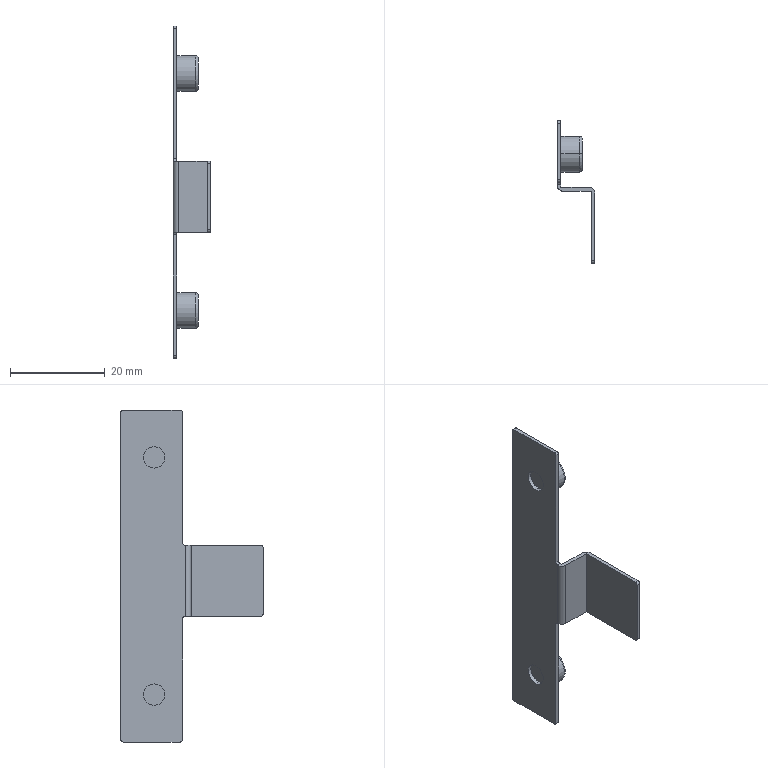Part | STEP file | 1 solid | 54 faces | box 8 x 30 x 70 mm | volume 1347 mm3 | plane 32 | cylinder 18 | torus 4 | commonest cylinder face diameters 1 x8 4.5 x4 7.5 x4 2.4 x2
STEP:
#1=CARTESIAN_POINT('',(4.8,-7.,-6.25));
#2=VERTEX_POINT('',#1);
#3=CARTESIAN_POINT('',(4.8,-7.,-13.75));
#4=VERTEX_POINT('',#3);
#5=CARTESIAN_POINT('',(4.8,-7.,-10.));
#6=DIRECTION('',(-1.,0.,0.));
#7=DIRECTION('',(0.,0.,-1.));
#8=AXIS2_PLACEMENT_3D('',#5,#6,#7);
#9=CIRCLE('',#8,3.75);
#10=EDGE_CURVE('',#2,#4,#9,.T.);
#11=ORIENTED_EDGE('',*,*,#10,.F.);
#12=CARTESIAN_POINT('',(5.3,-7.,-6.75));
#13=VERTEX_POINT('',#12);
#14=CARTESIAN_POINT('',(4.8,-7.,-6.75));
#15=DIRECTION('',(0.,1.,0.));
#16=DIRECTION('',(0.,0.,1.));
#17=AXIS2_PLACEMENT_3D('',#14,#15,#16);
#18=CIRCLE('',#17,0.5);
#19=EDGE_CURVE('',#2,#13,#18,.T.);
#20=ORIENTED_EDGE('',*,*,#19,.T.);
#21=CARTESIAN_POINT('',(5.3,-7.,-13.25));
#22=VERTEX_POINT('',#21);
#23=CARTESIAN_POINT('',(5.3,-7.,-10.));
#24=DIRECTION('',(1.,0.,0.));
#25=DIRECTION('',(0.,0.,-1.));
#26=AXIS2_PLACEMENT_3D('',#23,#24,#25);
#27=CIRCLE('',#26,3.25);
#28=EDGE_CURVE('',#22,#13,#27,.T.);
#29=ORIENTED_EDGE('',*,*,#28,.F.);
#30=CARTESIAN_POINT('',(4.8,-7.,-13.25));
#31=DIRECTION('',(0.,-1.,0.));
#32=DIRECTION('',(0.,0.,-1.));
#33=AXIS2_PLACEMENT_3D('',#30,#31,#32);
#34=CIRCLE('',#33,0.5);
#35=EDGE_CURVE('',#4,#22,#34,.T.);
#36=ORIENTED_EDGE('',*,*,#35,.F.);
#37=EDGE_LOOP('',(#11,#20,#29,#36));
#38=FACE_OUTER_BOUND('',#37,.T.);
#39=CARTESIAN_POINT('',(4.8,-7.,-10.));
#40=DIRECTION('',(1.,0.,0.));
#41=DIRECTION('',(0.,0.,-1.));
#42=AXIS2_PLACEMENT_3D('',#39,#40,#41);
#43=TOROIDAL_SURFACE('',#42,3.25,0.5);
#44=ADVANCED_FACE('',(#38),#43,.T.);
#45=CARTESIAN_POINT('',(4.8,-7.,-56.25));
#46=VERTEX_POINT('',#45);
#47=CARTESIAN_POINT('',(4.8,-7.,-63.75));
#48=VERTEX_POINT('',#47);
#49=CARTESIAN_POINT('',(4.8,-7.,-60.));
#50=DIRECTION('',(-1.,0.,0.));
#51=DIRECTION('',(0.,0.,-1.));
#52=AXIS2_PLACEMENT_3D('',#49,#50,#51);
#53=CIRCLE('',#52,3.75);
#54=EDGE_CURVE('',#46,#48,#53,.T.);
#55=ORIENTED_EDGE('',*,*,#54,.F.);
#56=CARTESIAN_POINT('',(5.3,-7.,-56.75));
#57=VERTEX_POINT('',#56);
#58=CARTESIAN_POINT('',(4.8,-7.,-56.75));
#59=DIRECTION('',(0.,1.,0.));
#60=DIRECTION('',(0.,0.,1.));
#61=AXIS2_PLACEMENT_3D('',#58,#59,#60);
#62=CIRCLE('',#61,0.5);
#63=EDGE_CURVE('',#46,#57,#62,.T.);
#64=ORIENTED_EDGE('',*,*,#63,.T.);
#65=CARTESIAN_POINT('',(5.3,-7.,-63.25));
#66=VERTEX_POINT('',#65);
#67=CARTESIAN_POINT('',(5.3,-7.,-60.));
#68=DIRECTION('',(1.,0.,0.));
#69=DIRECTION('',(0.,0.,-1.));
#70=AXIS2_PLACEMENT_3D('',#67,#68,#69);
#71=CIRCLE('',#70,3.25);
#72=EDGE_CURVE('',#66,#57,#71,.T.);
#73=ORIENTED_EDGE('',*,*,#72,.F.);
#74=CARTESIAN_POINT('',(4.8,-7.,-63.25));
#75=DIRECTION('',(0.,-1.,0.));
#76=DIRECTION('',(0.,0.,-1.));
#77=AXIS2_PLACEMENT_3D('',#74,#75,#76);
#78=CIRCLE('',#77,0.5);
#79=EDGE_CURVE('',#48,#66,#78,.T.);
#80=ORIENTED_EDGE('',*,*,#79,.F.);
#81=EDGE_LOOP('',(#55,#64,#73,#80));
#82=FACE_OUTER_BOUND('',#81,.T.);
#83=CARTESIAN_POINT('',(4.8,-7.,-60.));
#84=DIRECTION('',(1.,0.,0.));
#85=DIRECTION('',(0.,0.,-1.));
#86=AXIS2_PLACEMENT_3D('',#83,#84,#85);
#87=TOROIDAL_SURFACE('',#86,3.25,0.5);
#88=ADVANCED_FACE('',(#82),#87,.T.);
#89=ORIENTED_EDGE('',*,*,#54,.T.);
#90=CARTESIAN_POINT('',(0.8,-7.,-63.75));
#91=VERTEX_POINT('',#90);
#92=CARTESIAN_POINT('',(5.3,-7.,-63.75));
#93=DIRECTION('',(-1.,0.,0.));
#94=VECTOR('',#93,1000.);
#95=LINE('',#92,#94);
#96=EDGE_CURVE('',#48,#91,#95,.T.);
#97=ORIENTED_EDGE('',*,*,#96,.T.);
#98=CARTESIAN_POINT('',(0.8,-7.,-56.25));
#99=VERTEX_POINT('',#98);
#100=CARTESIAN_POINT('',(0.8,-7.,-60.));
#101=DIRECTION('',(1.,0.,0.));
#102=DIRECTION('',(0.,0.,-1.));
#103=AXIS2_PLACEMENT_3D('',#100,#101,#102);
#104=CIRCLE('',#103,3.75);
#105=EDGE_CURVE('',#91,#99,#104,.T.);
#106=ORIENTED_EDGE('',*,*,#105,.T.);
#107=CARTESIAN_POINT('',(5.3,-7.,-56.25));
#108=DIRECTION('',(-1.,0.,0.));
#109=VECTOR('',#108,1000.);
#110=LINE('',#107,#109);
#111=EDGE_CURVE('',#46,#99,#110,.T.);
#112=ORIENTED_EDGE('',*,*,#111,.F.);
#113=EDGE_LOOP('',(#89,#97,#106,#112));
#114=FACE_OUTER_BOUND('',#113,.T.);
#115=CARTESIAN_POINT('',(5.3,-7.,-60.));
#116=DIRECTION('',(-1.,0.,0.));
#117=DIRECTION('',(0.,0.,1.));
#118=AXIS2_PLACEMENT_3D('',#115,#116,#117);
#119=CYLINDRICAL_SURFACE('',#118,3.75);
#120=ADVANCED_FACE('',(#114),#119,.T.);
#121=ORIENTED_EDGE('',*,*,#10,.T.);
#122=CARTESIAN_POINT('',(0.8,-7.,-13.75));
#123=VERTEX_POINT('',#122);
#124=CARTESIAN_POINT('',(5.3,-7.,-13.75));
#125=DIRECTION('',(-1.,0.,0.));
#126=VECTOR('',#125,1000.);
#127=LINE('',#124,#126);
#128=EDGE_CURVE('',#4,#123,#127,.T.);
#129=ORIENTED_EDGE('',*,*,#128,.T.);
#130=CARTESIAN_POINT('',(0.8,-7.,-6.25));
#131=VERTEX_POINT('',#130);
#132=CARTESIAN_POINT('',(0.8,-7.,-10.));
#133=DIRECTION('',(1.,0.,0.));
#134=DIRECTION('',(0.,0.,-1.));
#135=AXIS2_PLACEMENT_3D('',#132,#133,#134);
#136=CIRCLE('',#135,3.75);
#137=EDGE_CURVE('',#123,#131,#136,.T.);
#138=ORIENTED_EDGE('',*,*,#137,.T.);
#139=CARTESIAN_POINT('',(5.3,-7.,-6.25));
#140=DIRECTION('',(-1.,0.,0.));
#141=VECTOR('',#140,1000.);
#142=LINE('',#139,#141);
#143=EDGE_CURVE('',#2,#131,#142,.T.);
#144=ORIENTED_EDGE('',*,*,#143,.F.);
#145=EDGE_LOOP('',(#121,#129,#138,#144));
#146=FACE_OUTER_BOUND('',#145,.T.);
#147=CARTESIAN_POINT('',(5.3,-7.,-10.));
#148=DIRECTION('',(-1.,0.,0.));
#149=DIRECTION('',(0.,0.,1.));
#150=AXIS2_PLACEMENT_3D('',#147,#148,#149);
#151=CYLINDRICAL_SURFACE('',#150,3.75);
#152=ADVANCED_FACE('',(#146),#151,.T.);
#153=CARTESIAN_POINT('',(0.8,-7.,-62.25));
#154=VERTEX_POINT('',#153);
#155=CARTESIAN_POINT('',(0.8,-7.,-57.75));
#156=VERTEX_POINT('',#155);
#157=CARTESIAN_POINT('',(0.8,-7.,-60.));
#158=DIRECTION('',(-1.,0.,0.));
#159=DIRECTION('',(0.,0.,1.));
#160=AXIS2_PLACEMENT_3D('',#157,#158,#159);
#161=CIRCLE('',#160,2.25);
#162=EDGE_CURVE('',#154,#156,#161,.T.);
#163=ORIENTED_EDGE('',*,*,#162,.F.);
#164=CARTESIAN_POINT('',(0.,-7.,-62.25));
#165=VERTEX_POINT('',#164);
#166=CARTESIAN_POINT('',(0.,-7.,-62.25));
#167=DIRECTION('',(-1.,0.,0.));
#168=VECTOR('',#167,1000.);
#169=LINE('',#166,#168);
#170=EDGE_CURVE('',#154,#165,#169,.T.);
#171=ORIENTED_EDGE('',*,*,#170,.T.);
#172=CARTESIAN_POINT('',(0.,-7.,-57.75));
#173=VERTEX_POINT('',#172);
#174=CARTESIAN_POINT('',(0.,-7.,-60.));
#175=DIRECTION('',(-1.,0.,0.));
#176=DIRECTION('',(0.,0.,1.));
#177=AXIS2_PLACEMENT_3D('',#174,#175,#176);
#178=CIRCLE('',#177,2.25);
#179=EDGE_CURVE('',#165,#173,#178,.T.);
#180=ORIENTED_EDGE('',*,*,#179,.T.);
#181=CARTESIAN_POINT('',(0.,-7.,-57.75));
#182=DIRECTION('',(-1.,0.,0.));
#183=VECTOR('',#182,1000.);
#184=LINE('',#181,#183);
#185=EDGE_CURVE('',#156,#173,#184,.T.);
#186=ORIENTED_EDGE('',*,*,#185,.F.);
#187=EDGE_LOOP('',(#163,#171,#180,#186));
#188=FACE_OUTER_BOUND('',#187,.T.);
#189=CARTESIAN_POINT('',(0.,-7.,-60.));
#190=DIRECTION('',(-1.,0.,0.));
#191=DIRECTION('',(0.,0.,1.));
#192=AXIS2_PLACEMENT_3D('',#189,#190,#191);
#193=CYLINDRICAL_SURFACE('',#192,2.25);
#194=ADVANCED_FACE('',(#188),#193,.F.);
#195=CARTESIAN_POINT('',(0.8,-7.,-12.25));
#196=VERTEX_POINT('',#195);
#197=CARTESIAN_POINT('',(0.8,-7.,-7.75));
#198=VERTEX_POINT('',#197);
#199=CARTESIAN_POINT('',(0.8,-7.,-10.));
#200=DIRECTION('',(-1.,0.,0.));
#201=DIRECTION('',(0.,0.,1.));
#202=AXIS2_PLACEMENT_3D('',#199,#200,#201);
#203=CIRCLE('',#202,2.25);
#204=EDGE_CURVE('',#196,#198,#203,.T.);
#205=ORIENTED_EDGE('',*,*,#204,.F.);
#206=CARTESIAN_POINT('',(0.,-7.,-12.25));
#207=VERTEX_POINT('',#206);
#208=CARTESIAN_POINT('',(0.,-7.,-12.25));
#209=DIRECTION('',(-1.,0.,0.));
#210=VECTOR('',#209,1000.);
#211=LINE('',#208,#210);
#212=EDGE_CURVE('',#196,#207,#211,.T.);
#213=ORIENTED_EDGE('',*,*,#212,.T.);
#214=CARTESIAN_POINT('',(0.,-7.,-7.75));
#215=VERTEX_POINT('',#214);
#216=CARTESIAN_POINT('',(0.,-7.,-10.));
#217=DIRECTION('',(-1.,0.,0.));
#218=DIRECTION('',(0.,0.,1.));
#219=AXIS2_PLACEMENT_3D('',#216,#217,#218);
#220=CIRCLE('',#219,2.25);
#221=EDGE_CURVE('',#207,#215,#220,.T.);
#222=ORIENTED_EDGE('',*,*,#221,.T.);
#223=CARTESIAN_POINT('',(0.,-7.,-7.75));
#224=DIRECTION('',(-1.,0.,0.));
#225=VECTOR('',#224,1000.);
#226=LINE('',#223,#225);
#227=EDGE_CURVE('',#198,#215,#226,.T.);
#228=ORIENTED_EDGE('',*,*,#227,.F.);
#229=EDGE_LOOP('',(#205,#213,#222,#228));
#230=FACE_OUTER_BOUND('',#229,.T.);
#231=CARTESIAN_POINT('',(0.,-7.,-10.));
#232=DIRECTION('',(-1.,0.,0.));
#233=DIRECTION('',(0.,0.,1.));
#234=AXIS2_PLACEMENT_3D('',#231,#232,#233);
#235=CYLINDRICAL_SURFACE('',#234,2.25);
#236=ADVANCED_FACE('',(#230),#235,.F.);
#237=CARTESIAN_POINT('',(0.,0.,-69.5));
#238=VERTEX_POINT('',#237);
#239=CARTESIAN_POINT('',(0.,0.,-0.5));
#240=VERTEX_POINT('',#239);
#241=CARTESIAN_POINT('',(0.,0.,-70.));
#242=DIRECTION('',(0.,0.,1.));
#243=VECTOR('',#242,1000.);
#244=LINE('',#241,#243);
#245=EDGE_CURVE('',#238,#240,#244,.T.);
#246=ORIENTED_EDGE('',*,*,#245,.T.);
#247=CARTESIAN_POINT('',(0.8,0.,-0.5));
#248=VERTEX_POINT('',#247);
#249=CARTESIAN_POINT('',(0.,0.,-0.5));
#250=DIRECTION('',(1.,0.,0.));
#251=VECTOR('',#250,1000.);
#252=LINE('',#249,#251);
#253=EDGE_CURVE('',#240,#248,#252,.T.);
#254=ORIENTED_EDGE('',*,*,#253,.T.);
#255=CARTESIAN_POINT('',(0.8,0.,-69.5));
#256=VERTEX_POINT('',#255);
#257=CARTESIAN_POINT('',(0.8,0.,-70.));
#258=DIRECTION('',(0.,0.,1.));
#259=VECTOR('',#258,1000.);
#260=LINE('',#257,#259);
#261=EDGE_CURVE('',#256,#248,#260,.T.);
#262=ORIENTED_EDGE('',*,*,#261,.F.);
#263=CARTESIAN_POINT('',(0.,0.,-69.5));
#264=DIRECTION('',(-1.,0.,0.));
#265=VECTOR('',#264,1000.);
#266=LINE('',#263,#265);
#267=EDGE_CURVE('',#256,#238,#266,.T.);
#268=ORIENTED_EDGE('',*,*,#267,.T.);
#269=EDGE_LOOP('',(#246,#254,#262,#268));
#270=FACE_OUTER_BOUND('',#269,.T.);
#271=CARTESIAN_POINT('',(0.,0.,-70.));
#272=DIRECTION('',(0.,1.,0.));
#273=DIRECTION('',(1.,0.,0.));
#274=AXIS2_PLACEMENT_3D('',#271,#272,#273);
#275=PLANE('',#274);
#276=ADVANCED_FACE('',(#270),#275,.T.);
#277=CARTESIAN_POINT('',(0.8,-12.5,-70.));
#278=VERTEX_POINT('',#277);
#279=CARTESIAN_POINT('',(0.8,-0.5,-70.));
#280=VERTEX_POINT('',#279);
#281=CARTESIAN_POINT('',(0.8,-30.,-70.));
#282=DIRECTION('',(0.,1.,0.));
#283=VECTOR('',#282,1000.);
#284=LINE('',#281,#283);
#285=EDGE_CURVE('',#278,#280,#284,.T.);
#286=ORIENTED_EDGE('',*,*,#285,.F.);
#287=CARTESIAN_POINT('',(0.,-12.5,-70.));
#288=VERTEX_POINT('',#287);
#289=CARTESIAN_POINT('',(0.,-12.5,-70.));
#290=DIRECTION('',(-1.,0.,0.));
#291=VECTOR('',#290,1000.);
#292=LINE('',#289,#291);
#293=EDGE_CURVE('',#278,#288,#292,.T.);
#294=ORIENTED_EDGE('',*,*,#293,.T.);
#295=CARTESIAN_POINT('',(0.,-0.5,-70.));
#296=VERTEX_POINT('',#295);
#297=CARTESIAN_POINT('',(0.,-30.,-70.));
#298=DIRECTION('',(0.,1.,0.));
#299=VECTOR('',#298,1000.);
#300=LINE('',#297,#299);
#301=EDGE_CURVE('',#288,#296,#300,.T.);
#302=ORIENTED_EDGE('',*,*,#301,.T.);
#303=CARTESIAN_POINT('',(0.,-0.5,-70.));
#304=DIRECTION('',(1.,0.,0.));
#305=VECTOR('',#304,1000.);
#306=LINE('',#303,#305);
#307=EDGE_CURVE('',#296,#280,#306,.T.);
#308=ORIENTED_EDGE('',*,*,#307,.T.);
#309=EDGE_LOOP('',(#286,#294,#302,#308));
#310=FACE_OUTER_BOUND('',#309,.T.);
#311=CARTESIAN_POINT('',(0.,-30.,-70.));
#312=DIRECTION('',(0.,0.,-1.));
#313=DIRECTION('',(0.,-1.,0.));
#314=AXIS2_PLACEMENT_3D('',#311,#312,#313);
#315=PLANE('',#314);
#316=ADVANCED_FACE('',(#310),#315,.T.);
#317=CARTESIAN_POINT('',(7.2,-30.,-43.));
#318=VERTEX_POINT('',#317);
#319=CARTESIAN_POINT('',(7.2,-30.,-29.));
#320=VERTEX_POINT('',#319);
#321=CARTESIAN_POINT('',(7.2,-30.,-70.));
#322=DIRECTION('',(0.,0.,1.));
#323=VECTOR('',#322,1000.);
#324=LINE('',#321,#323);
#325=EDGE_CURVE('',#318,#320,#324,.T.);
#326=ORIENTED_EDGE('',*,*,#325,.F.);
#327=CARTESIAN_POINT('',(8.,-30.,-43.));
#328=VERTEX_POINT('',#327);
#329=CARTESIAN_POINT('',(8.,-30.,-43.));
#330=DIRECTION('',(1.,0.,0.));
#331=VECTOR('',#330,1000.);
#332=LINE('',#329,#331);
#333=EDGE_CURVE('',#318,#328,#332,.T.);
#334=ORIENTED_EDGE('',*,*,#333,.T.);
#335=CARTESIAN_POINT('',(8.,-30.,-29.));
#336=VERTEX_POINT('',#335);
#337=CARTESIAN_POINT('',(8.,-30.,-43.5));
#338=DIRECTION('',(0.,0.,-1.));
#339=VECTOR('',#338,1000.);
#340=LINE('',#337,#339);
#341=EDGE_CURVE('',#336,#328,#340,.T.);
#342=ORIENTED_EDGE('',*,*,#341,.F.);
#343=CARTESIAN_POINT('',(7.2,-30.,-29.));
#344=DIRECTION('',(-1.,0.,0.));
#345=VECTOR('',#344,1000.);
#346=LINE('',#343,#345);
#347=EDGE_CURVE('',#336,#320,#346,.T.);
#348=ORIENTED_EDGE('',*,*,#347,.T.);
#349=EDGE_LOOP('',(#326,#334,#342,#348));
#350=FACE_OUTER_BOUND('',#349,.T.);
#351=CARTESIAN_POINT('',(0.,-30.,0.));
#352=DIRECTION('',(0.,-1.,0.));
#353=DIRECTION('',(0.,0.,-1.));
#354=AXIS2_PLACEMENT_3D('',#351,#352,#353);
#355=PLANE('',#354);
#356=ADVANCED_FACE('',(#350),#355,.T.);
#357=CARTESIAN_POINT('',(0.8,-0.5,0.));
#358=VERTEX_POINT('',#357);
#359=CARTESIAN_POINT('',(0.8,-12.5,0.));
#360=VERTEX_POINT('',#359);
#361=CARTESIAN_POINT('',(0.8,0.,0.));
#362=DIRECTION('',(0.,-1.,0.));
#363=VECTOR('',#362,1000.);
#364=LINE('',#361,#363);
#365=EDGE_CURVE('',#358,#360,#364,.T.);
#366=ORIENTED_EDGE('',*,*,#365,.F.);
#367=CARTESIAN_POINT('',(0.,-0.5,0.));
#368=VERTEX_POINT('',#367);
#369=CARTESIAN_POINT('',(0.,-0.5,0.));
#370=DIRECTION('',(-1.,0.,0.));
#371=VECTOR('',#370,1000.);
#372=LINE('',#369,#371);
#373=EDGE_CURVE('',#358,#368,#372,.T.);
#374=ORIENTED_EDGE('',*,*,#373,.T.);
#375=CARTESIAN_POINT('',(0.,-12.5,0.));
#376=VERTEX_POINT('',#375);
#377=CARTESIAN_POINT('',(0.,0.,0.));
#378=DIRECTION('',(0.,-1.,0.));
#379=VECTOR('',#378,1000.);
#380=LINE('',#377,#379);
#381=EDGE_CURVE('',#368,#376,#380,.T.);
#382=ORIENTED_EDGE('',*,*,#381,.T.);
#383=CARTESIAN_POINT('',(0.8,-12.5,0.));
#384=DIRECTION('',(1.,0.,0.));
#385=VECTOR('',#384,1000.);
#386=LINE('',#383,#385);
#387=EDGE_CURVE('',#376,#360,#386,.T.);
#388=ORIENTED_EDGE('',*,*,#387,.T.);
#389=EDGE_LOOP('',(#366,#374,#382,#388));
#390=FACE_OUTER_BOUND('',#389,.T.);
#391=CARTESIAN_POINT('',(0.,0.,0.));
#392=DIRECTION('',(0.,0.,1.));
#393=DIRECTION('',(1.,0.,0.));
#394=AXIS2_PLACEMENT_3D('',#391,#392,#393);
#395=PLANE('',#394);
#396=ADVANCED_FACE('',(#390),#395,.T.);
#397=CARTESIAN_POINT('',(0.,-13.6,-43.5));
#398=VERTEX_POINT('',#397);
#399=CARTESIAN_POINT('',(0.,-13.5,-43.5));
#400=VERTEX_POINT('',#399);
#401=CARTESIAN_POINT('',(0.,-30.,-43.5));
#402=DIRECTION('',(0.,1.,0.));
#403=VECTOR('',#402,1000.);
#404=LINE('',#401,#403);
#405=EDGE_CURVE('',#398,#400,#404,.T.);
#406=ORIENTED_EDGE('',*,*,#405,.F.);
#407=CARTESIAN_POINT('',(0.,-13.6,-28.5));
#408=VERTEX_POINT('',#407);
#409=CARTESIAN_POINT('',(0.,-13.6,0.));
#410=DIRECTION('',(0.,0.,1.));
#411=VECTOR('',#410,1000.);
#412=LINE('',#409,#411);
#413=EDGE_CURVE('',#398,#408,#412,.T.);
#414=ORIENTED_EDGE('',*,*,#413,.T.);
#415=CARTESIAN_POINT('',(0.,-13.5,-28.5));
#416=VERTEX_POINT('',#415);
#417=CARTESIAN_POINT('',(0.,-13.,-28.5));
#418=DIRECTION('',(0.,-1.,0.));
#419=VECTOR('',#418,1000.);
#420=LINE('',#417,#419);
#421=EDGE_CURVE('',#416,#408,#420,.T.);
#422=ORIENTED_EDGE('',*,*,#421,.F.);
#423=CARTESIAN_POINT('',(0.,-13.,-28.));
#424=VERTEX_POINT('',#423);
#425=CARTESIAN_POINT('',(0.,-13.5,-28.));
#426=DIRECTION('',(1.,0.,0.));
#427=DIRECTION('',(0.,0.,-1.));
#428=AXIS2_PLACEMENT_3D('',#425,#426,#427);
#429=CIRCLE('',#428,0.5);
#430=EDGE_CURVE('',#416,#424,#429,.T.);
#431=ORIENTED_EDGE('',*,*,#430,.T.);
#432=CARTESIAN_POINT('',(0.,-13.,-0.5));
#433=VERTEX_POINT('',#432);
#434=CARTESIAN_POINT('',(0.,-13.,0.));
#435=DIRECTION('',(0.,0.,-1.));
#436=VECTOR('',#435,1000.);
#437=LINE('',#434,#436);
#438=EDGE_CURVE('',#433,#424,#437,.T.);
#439=ORIENTED_EDGE('',*,*,#438,.F.);
#440=CARTESIAN_POINT('',(0.,-12.5,-0.5));
#441=DIRECTION('',(-1.,0.,0.));
#442=DIRECTION('',(0.,0.,-1.));
#443=AXIS2_PLACEMENT_3D('',#440,#441,#442);
#444=CIRCLE('',#443,0.5);
#445=EDGE_CURVE('',#433,#376,#444,.T.);
#446=ORIENTED_EDGE('',*,*,#445,.T.);
#447=ORIENTED_EDGE('',*,*,#381,.F.);
#448=CARTESIAN_POINT('',(0.,-0.5,-0.5));
#449=DIRECTION('',(-1.,0.,0.));
#450=DIRECTION('',(0.,0.,-1.));
#451=AXIS2_PLACEMENT_3D('',#448,#449,#450);
#452=CIRCLE('',#451,0.5);
#453=EDGE_CURVE('',#368,#240,#452,.T.);
#454=ORIENTED_EDGE('',*,*,#453,.T.);
#455=ORIENTED_EDGE('',*,*,#245,.F.);
#456=CARTESIAN_POINT('',(0.,-0.5,-69.5));
#457=DIRECTION('',(-1.,0.,0.));
#458=DIRECTION('',(0.,0.,-1.));
#459=AXIS2_PLACEMENT_3D('',#456,#457,#458);
#460=CIRCLE('',#459,0.5);
#461=EDGE_CURVE('',#238,#296,#460,.T.);
#462=ORIENTED_EDGE('',*,*,#461,.T.);
#463=ORIENTED_EDGE('',*,*,#301,.F.);
#464=CARTESIAN_POINT('',(0.,-13.,-69.5));
#465=VERTEX_POINT('',#464);
#466=CARTESIAN_POINT('',(0.,-12.5,-69.5));
#467=DIRECTION('',(-1.,0.,0.));
#468=DIRECTION('',(0.,0.,-1.));
#469=AXIS2_PLACEMENT_3D('',#466,#467,#468);
#470=CIRCLE('',#469,0.5);
#471=EDGE_CURVE('',#288,#465,#470,.T.);
#472=ORIENTED_EDGE('',*,*,#471,.T.);
#473=CARTESIAN_POINT('',(0.,-13.,-44.));
#474=VERTEX_POINT('',#473);
#475=CARTESIAN_POINT('',(0.,-13.,-43.5));
#476=DIRECTION('',(0.,0.,-1.));
#477=VECTOR('',#476,1000.);
#478=LINE('',#475,#477);
#479=EDGE_CURVE('',#474,#465,#478,.T.);
#480=ORIENTED_EDGE('',*,*,#479,.F.);
#481=CARTESIAN_POINT('',(0.,-13.5,-44.));
#482=DIRECTION('',(1.,0.,0.));
#483=DIRECTION('',(0.,0.,-1.));
#484=AXIS2_PLACEMENT_3D('',#481,#482,#483);
#485=CIRCLE('',#484,0.5);
#486=EDGE_CURVE('',#474,#400,#485,.T.);
#487=ORIENTED_EDGE('',*,*,#486,.T.);
#488=EDGE_LOOP('',(#406,#414,#422,#431,#439,#446,#447,#454,#455,#462,#463,#472,#480,#487));
#489=FACE_OUTER_BOUND('',#488,.T.);
#490=CARTESIAN_POINT('',(0.,-7.,-60.));
#491=DIRECTION('',(-1.,0.,0.));
#492=DIRECTION('',(0.,0.,1.));
#493=AXIS2_PLACEMENT_3D('',#490,#491,#492);
#494=CIRCLE('',#493,2.25);
#495=EDGE_CURVE('',#173,#165,#494,.T.);
#496=ORIENTED_EDGE('',*,*,#495,.F.);
#497=ORIENTED_EDGE('',*,*,#179,.F.);
#498=EDGE_LOOP('',(#496,#497));
#499=FACE_BOUND('',#498,.T.);
#500=CARTESIAN_POINT('',(0.,-7.,-10.));
#501=DIRECTION('',(-1.,0.,0.));
#502=DIRECTION('',(0.,0.,1.));
#503=AXIS2_PLACEMENT_3D('',#500,#501,#502);
#504=CIRCLE('',#503,2.25);
#505=EDGE_CURVE('',#215,#207,#504,.T.);
#506=ORIENTED_EDGE('',*,*,#505,.F.);
#507=ORIENTED_EDGE('',*,*,#221,.F.);
#508=EDGE_LOOP('',(#506,#507));
#509=FACE_BOUND('',#508,.T.);
#510=CARTESIAN_POINT('',(0.,0.,0.));
#511=DIRECTION('',(1.,0.,0.));
#512=DIRECTION('',(0.,1.,0.));
#513=AXIS2_PLACEMENT_3D('',#510,#511,#512);
#514=PLANE('',#513);
#515=ADVANCED_FACE('',(#489,#499,#509),#514,.F.);
#516=ORIENTED_EDGE('',*,*,#261,.T.);
#517=CARTESIAN_POINT('',(0.8,-0.5,-0.5));
#518=DIRECTION('',(1.,0.,0.));
#519=DIRECTION('',(0.,0.,-1.));
#520=AXIS2_PLACEMENT_3D('',#517,#518,#519);
#521=CIRCLE('',#520,0.5);
#522=EDGE_CURVE('',#248,#358,#521,.T.);
#523=ORIENTED_EDGE('',*,*,#522,.T.);
#524=ORIENTED_EDGE('',*,*,#365,.T.);
#525=CARTESIAN_POINT('',(0.8,-13.,-0.5));
#526=VERTEX_POINT('',#525);
#527=CARTESIAN_POINT('',(0.8,-12.5,-0.5));
#528=DIRECTION('',(1.,0.,0.));
#529=DIRECTION('',(0.,0.,-1.));
#530=AXIS2_PLACEMENT_3D('',#527,#528,#529);
#531=CIRCLE('',#530,0.5);
#532=EDGE_CURVE('',#360,#526,#531,.T.);
#533=ORIENTED_EDGE('',*,*,#532,.T.);
#534=CARTESIAN_POINT('',(0.8,-13.,-28.));
#535=VERTEX_POINT('',#534);
#536=CARTESIAN_POINT('',(0.8,-13.,0.));
#537=DIRECTION('',(0.,0.,-1.));
#538=VECTOR('',#537,1000.);
#539=LINE('',#536,#538);
#540=EDGE_CURVE('',#526,#535,#539,.T.);
#541=ORIENTED_EDGE('',*,*,#540,.T.);
#542=CARTESIAN_POINT('',(0.8,-13.5,-28.5));
#543=VERTEX_POINT('',#542);
#544=CARTESIAN_POINT('',(0.8,-13.5,-28.));
#545=DIRECTION('',(-1.,0.,0.));
#546=DIRECTION('',(0.,0.,-1.));
#547=AXIS2_PLACEMENT_3D('',#544,#545,#546);
#548=CIRCLE('',#547,0.5);
#549=EDGE_CURVE('',#535,#543,#548,.T.);
#550=ORIENTED_EDGE('',*,*,#549,.T.);
#551=CARTESIAN_POINT('',(0.8,-14.,-28.5));
#552=VERTEX_POINT('',#551);
#553=CARTESIAN_POINT('',(0.8,-13.,-28.5));
#554=DIRECTION('',(0.,-1.,0.));
#555=VECTOR('',#554,1000.);
#556=LINE('',#553,#555);
#557=EDGE_CURVE('',#543,#552,#556,.T.);
#558=ORIENTED_EDGE('',*,*,#557,.T.);
#559=CARTESIAN_POINT('',(0.8,-14.,-43.5));
#560=VERTEX_POINT('',#559);
#561=CARTESIAN_POINT('',(0.8,-14.,-28.5));
#562=DIRECTION('',(0.,0.,1.));
#563=VECTOR('',#562,1000.);
#564=LINE('',#561,#563);
#565=EDGE_CURVE('',#560,#552,#564,.T.);
#566=ORIENTED_EDGE('',*,*,#565,.F.);
#567=CARTESIAN_POINT('',(0.8,-13.5,-43.5));
#568=VERTEX_POINT('',#567);
#569=CARTESIAN_POINT('',(0.8,-30.,-43.5));
#570=DIRECTION('',(0.,1.,0.));
#571=VECTOR('',#570,1000.);
#572=LINE('',#569,#571);
#573=EDGE_CURVE('',#560,#568,#572,.T.);
#574=ORIENTED_EDGE('',*,*,#573,.T.);
#575=CARTESIAN_POINT('',(0.8,-13.,-44.));
#576=VERTEX_POINT('',#575);
#577=CARTESIAN_POINT('',(0.8,-13.5,-44.));
#578=DIRECTION('',(-1.,0.,0.));
#579=DIRECTION('',(0.,0.,-1.));
#580=AXIS2_PLACEMENT_3D('',#577,#578,#579);
#581=CIRCLE('',#580,0.5);
#582=EDGE_CURVE('',#568,#576,#581,.T.);
#583=ORIENTED_EDGE('',*,*,#582,.T.);
#584=CARTESIAN_POINT('',(0.8,-13.,-69.5));
#585=VERTEX_POINT('',#584);
#586=CARTESIAN_POINT('',(0.8,-13.,-43.5));
#587=DIRECTION('',(0.,0.,-1.));
#588=VECTOR('',#587,1000.);
#589=LINE('',#586,#588);
#590=EDGE_CURVE('',#576,#585,#589,.T.);
#591=ORIENTED_EDGE('',*,*,#590,.T.);
#592=CARTESIAN_POINT('',(0.8,-12.5,-69.5));
#593=DIRECTION('',(1.,0.,0.));
#594=DIRECTION('',(0.,0.,-1.));
#595=AXIS2_PLACEMENT_3D('',#592,#593,#594);
#596=CIRCLE('',#595,0.5);
#597=EDGE_CURVE('',#585,#278,#596,.T.);
#598=ORIENTED_EDGE('',*,*,#597,.T.);
#599=ORIENTED_EDGE('',*,*,#285,.T.);
#600=CARTESIAN_POINT('',(0.8,-0.5,-69.5));
#601=DIRECTION('',(1.,0.,0.));
#602=DIRECTION('',(0.,0.,-1.));
#603=AXIS2_PLACEMENT_3D('',#600,#601,#602);
#604=CIRCLE('',#603,0.5);
#605=EDGE_CURVE('',#280,#256,#604,.T.);
#606=ORIENTED_EDGE('',*,*,#605,.T.);
#607=EDGE_LOOP('',(#516,#523,#524,#533,#541,#550,#558,#566,#574,#583,#591,#598,#599,#606));
#608=FACE_OUTER_BOUND('',#607,.T.);
#609=CARTESIAN_POINT('',(0.8,-7.,-60.));
#610=DIRECTION('',(1.,0.,0.));
#611=DIRECTION('',(0.,0.,-1.));
#612=AXIS2_PLACEMENT_3D('',#609,#610,#611);
#613=CIRCLE('',#612,3.75);
#614=EDGE_CURVE('',#99,#91,#613,.T.);
#615=ORIENTED_EDGE('',*,*,#614,.F.);
#616=ORIENTED_EDGE('',*,*,#105,.F.);
#617=EDGE_LOOP('',(#615,#616));
#618=FACE_BOUND('',#617,.T.);
#619=CARTESIAN_POINT('',(0.8,-7.,-10.));
#620=DIRECTION('',(1.,0.,0.));
#621=DIRECTION('',(0.,0.,-1.));
#622=AXIS2_PLACEMENT_3D('',#619,#620,#621);
#623=CIRCLE('',#622,3.75);
#624=EDGE_CURVE('',#131,#123,#623,.T.);
#625=ORIENTED_EDGE('',*,*,#624,.F.);
#626=ORIENTED_EDGE('',*,*,#137,.F.);
#627=EDGE_LOOP('',(#625,#626));
#628=FACE_BOUND('',#627,.T.);
#629=CARTESIAN_POINT('',(0.8,0.,0.));
#630=DIRECTION('',(1.,0.,0.));
#631=DIRECTION('',(0.,1.,0.));
#632=AXIS2_PLACEMENT_3D('',#629,#630,#631);
#633=PLANE('',#632);
#634=ADVANCED_FACE('',(#608,#618,#628),#633,.T.);
#635=ORIENTED_EDGE('',*,*,#421,.T.);
#636=CARTESIAN_POINT('',(1.2,-14.8,-28.5));
#637=VERTEX_POINT('',#636);
#638=CARTESIAN_POINT('',(1.2,-13.6,-28.5));
#639=DIRECTION('',(0.,0.,1.));
#640=DIRECTION('',(-1.,0.,0.));
#641=AXIS2_PLACEMENT_3D('',#638,#639,#640);
#642=CIRCLE('',#641,1.2);
#643=EDGE_CURVE('',#408,#637,#642,.T.);
#644=ORIENTED_EDGE('',*,*,#643,.T.);
#645=CARTESIAN_POINT('',(7.2,-14.8,-28.5));
#646=VERTEX_POINT('',#645);
#647=CARTESIAN_POINT('',(7.2,-14.8,-28.5));
#648=DIRECTION('',(-1.,0.,0.));
#649=VECTOR('',#648,1000.);
#650=LINE('',#647,#649);
#651=EDGE_CURVE('',#646,#637,#650,.T.);
#652=ORIENTED_EDGE('',*,*,#651,.F.);
#653=CARTESIAN_POINT('',(7.2,-29.5,-28.5));
#654=VERTEX_POINT('',#653);
#655=CARTESIAN_POINT('',(7.2,-30.,-28.5));
#656=DIRECTION('',(0.,1.,0.));
#657=VECTOR('',#656,1000.);
#658=LINE('',#655,#657);
#659=EDGE_CURVE('',#654,#646,#658,.T.);
#660=ORIENTED_EDGE('',*,*,#659,.F.);
#661=CARTESIAN_POINT('',(8.,-29.5,-28.5));
#662=VERTEX_POINT('',#661);
#663=CARTESIAN_POINT('',(8.,-29.5,-28.5));
#664=DIRECTION('',(1.,0.,0.));
#665=VECTOR('',#664,1000.);
#666=LINE('',#663,#665);
#667=EDGE_CURVE('',#654,#662,#666,.T.);
#668=ORIENTED_EDGE('',*,*,#667,.T.);
#669=CARTESIAN_POINT('',(8.,-15.2,-28.5));
#670=VERTEX_POINT('',#669);
#671=CARTESIAN_POINT('',(8.,-30.,-28.5));
#672=DIRECTION('',(0.,-1.,0.));
#673=VECTOR('',#672,1000.);
#674=LINE('',#671,#673);
#675=EDGE_CURVE('',#670,#662,#674,.T.);
#676=ORIENTED_EDGE('',*,*,#675,.F.);
#677=CARTESIAN_POINT('',(6.8,-14.,-28.5));
#678=VERTEX_POINT('',#677);
#679=CARTESIAN_POINT('',(6.8,-15.2,-28.5));
#680=DIRECTION('',(0.,0.,1.));
#681=DIRECTION('',(-1.,0.,0.));
#682=AXIS2_PLACEMENT_3D('',#679,#680,#681);
#683=CIRCLE('',#682,1.2);
#684=EDGE_CURVE('',#670,#678,#683,.T.);
#685=ORIENTED_EDGE('',*,*,#684,.T.);
#686=CARTESIAN_POINT('',(8.,-14.,-28.5));
#687=DIRECTION('',(-1.,0.,0.));
#688=VECTOR('',#687,1000.);
#689=LINE('',#686,#688);
#690=EDGE_CURVE('',#678,#552,#689,.T.);
#691=ORIENTED_EDGE('',*,*,#690,.T.);
#692=ORIENTED_EDGE('',*,*,#557,.F.);
#693=CARTESIAN_POINT('',(0.,-13.5,-28.5));
#694=DIRECTION('',(-1.,0.,0.));
#695=VECTOR('',#694,1000.);
#696=LINE('',#693,#695);
#697=EDGE_CURVE('',#543,#416,#696,.T.);
#698=ORIENTED_EDGE('',*,*,#697,.T.);
#699=EDGE_LOOP('',(#635,#644,#652,#660,#668,#676,#685,#691,#692,#698));
#700=FACE_OUTER_BOUND('',#699,.T.);
#701=CARTESIAN_POINT('',(0.8,-13.,-28.5));
#702=DIRECTION('',(0.,0.,-1.));
#703=DIRECTION('',(0.,-1.,0.));
#704=AXIS2_PLACEMENT_3D('',#701,#702,#703);
#705=PLANE('',#704);
#706=ADVANCED_FACE('',(#700),#705,.F.);
#707=ORIENTED_EDGE('',*,*,#438,.T.);
#708=CARTESIAN_POINT('',(0.8,-13.,-28.));
#709=DIRECTION('',(1.,0.,0.));
#710=VECTOR('',#709,1000.);
#711=LINE('',#708,#710);
#712=EDGE_CURVE('',#424,#535,#711,.T.);
#713=ORIENTED_EDGE('',*,*,#712,.T.);
#714=ORIENTED_EDGE('',*,*,#540,.F.);
#715=CARTESIAN_POINT('',(0.,-13.,-0.5));
#716=DIRECTION('',(-1.,0.,0.));
#717=VECTOR('',#716,1000.);
#718=LINE('',#715,#717);
#719=EDGE_CURVE('',#526,#433,#718,.T.);
#720=ORIENTED_EDGE('',*,*,#719,.T.);
#721=EDGE_LOOP('',(#707,#713,#714,#720));
#722=FACE_OUTER_BOUND('',#721,.T.);
#723=CARTESIAN_POINT('',(0.8,-13.,0.));
#724=DIRECTION('',(0.,1.,0.));
#725=DIRECTION('',(1.,0.,0.));
#726=AXIS2_PLACEMENT_3D('',#723,#724,#725);
#727=PLANE('',#726);
#728=ADVANCED_FACE('',(#722),#727,.F.);
#729=ORIENTED_EDGE('',*,*,#479,.T.);
#730=CARTESIAN_POINT('',(0.8,-13.,-69.5));
#731=DIRECTION('',(1.,0.,0.));
#732=VECTOR('',#731,1000.);
#733=LINE('',#730,#732);
#734=EDGE_CURVE('',#465,#585,#733,.T.);
#735=ORIENTED_EDGE('',*,*,#734,.T.);
#736=ORIENTED_EDGE('',*,*,#590,.F.);
#737=CARTESIAN_POINT('',(0.,-13.,-44.));
#738=DIRECTION('',(-1.,0.,0.));
#739=VECTOR('',#738,1000.);
#740=LINE('',#737,#739);
#741=EDGE_CURVE('',#576,#474,#740,.T.);
#742=ORIENTED_EDGE('',*,*,#741,.T.);
#743=EDGE_LOOP('',(#729,#735,#736,#742));
#744=FACE_OUTER_BOUND('',#743,.T.);
#745=CARTESIAN_POINT('',(0.8,-13.,-43.5));
#746=DIRECTION('',(0.,1.,0.));
#747=DIRECTION('',(1.,0.,0.));
#748=AXIS2_PLACEMENT_3D('',#745,#746,#747);
#749=PLANE('',#748);
#750=ADVANCED_FACE('',(#744),#749,.F.);
#751=CARTESIAN_POINT('',(7.2,-14.8,-43.5));
#752=VERTEX_POINT('',#751);
#753=CARTESIAN_POINT('',(1.2,-14.8,-43.5));
#754=VERTEX_POINT('',#753);
#755=CARTESIAN_POINT('',(0.8,-14.8,-43.5));
#756=DIRECTION('',(-1.,0.,0.));
#757=VECTOR('',#756,1000.);
#758=LINE('',#755,#757);
#759=EDGE_CURVE('',#752,#754,#758,.T.);
#760=ORIENTED_EDGE('',*,*,#759,.T.);
#761=CARTESIAN_POINT('',(1.2,-13.6,-43.5));
#762=DIRECTION('',(0.,0.,-1.));
#763=DIRECTION('',(1.,0.,0.));
#764=AXIS2_PLACEMENT_3D('',#761,#762,#763);
#765=CIRCLE('',#764,1.2);
#766=EDGE_CURVE('',#754,#398,#765,.T.);
#767=ORIENTED_EDGE('',*,*,#766,.T.);
#768=ORIENTED_EDGE('',*,*,#405,.T.);
#769=CARTESIAN_POINT('',(0.8,-13.5,-43.5));
#770=DIRECTION('',(1.,0.,0.));
#771=VECTOR('',#770,1000.);
#772=LINE('',#769,#771);
#773=EDGE_CURVE('',#400,#568,#772,.T.);
#774=ORIENTED_EDGE('',*,*,#773,.T.);
#775=ORIENTED_EDGE('',*,*,#573,.F.);
#776=CARTESIAN_POINT('',(6.8,-14.,-43.5));
#777=VERTEX_POINT('',#776);
#778=CARTESIAN_POINT('',(8.,-14.,-43.5));
#779=DIRECTION('',(-1.,0.,0.));
#780=VECTOR('',#779,1000.);
#781=LINE('',#778,#780);
#782=EDGE_CURVE('',#777,#560,#781,.T.);
#783=ORIENTED_EDGE('',*,*,#782,.F.);
#784=CARTESIAN_POINT('',(8.,-15.2,-43.5));
#785=VERTEX_POINT('',#784);
#786=CARTESIAN_POINT('',(6.8,-15.2,-43.5));
#787=DIRECTION('',(0.,0.,-1.));
#788=DIRECTION('',(1.,0.,0.));
#789=AXIS2_PLACEMENT_3D('',#786,#787,#788);
#790=CIRCLE('',#789,1.2);
#791=EDGE_CURVE('',#777,#785,#790,.T.);
#792=ORIENTED_EDGE('',*,*,#791,.T.);
#793=CARTESIAN_POINT('',(8.,-29.5,-43.5));
#794=VERTEX_POINT('',#793);
#795=CARTESIAN_POINT('',(8.,-14.,-43.5));
#796=DIRECTION('',(0.,1.,0.));
#797=VECTOR('',#796,1000.);
#798=LINE('',#795,#797);
#799=EDGE_CURVE('',#794,#785,#798,.T.);
#800=ORIENTED_EDGE('',*,*,#799,.F.);
#801=CARTESIAN_POINT('',(7.2,-29.5,-43.5));
#802=VERTEX_POINT('',#801);
#803=CARTESIAN_POINT('',(7.2,-29.5,-43.5));
#804=DIRECTION('',(-1.,0.,0.));
#805=VECTOR('',#804,1000.);
#806=LINE('',#803,#805);
#807=EDGE_CURVE('',#794,#802,#806,.T.);
#808=ORIENTED_EDGE('',*,*,#807,.T.);
#809=CARTESIAN_POINT('',(7.2,-30.,-43.5));
#810=DIRECTION('',(0.,1.,0.));
#811=VECTOR('',#810,1000.);
#812=LINE('',#809,#811);
#813=EDGE_CURVE('',#802,#752,#812,.T.);
#814=ORIENTED_EDGE('',*,*,#813,.T.);
#815=EDGE_LOOP('',(#760,#767,#768,#774,#775,#783,#792,#800,#808,#814));
#816=FACE_OUTER_BOUND('',#815,.T.);
#817=CARTESIAN_POINT('',(0.8,-30.,-43.5));
#818=DIRECTION('',(0.,0.,1.));
#819=DIRECTION('',(1.,0.,0.));
#820=AXIS2_PLACEMENT_3D('',#817,#818,#819);
#821=PLANE('',#820);
#822=ADVANCED_FACE('',(#816),#821,.F.);
#823=ORIENTED_EDGE('',*,*,#690,.F.);
#824=CARTESIAN_POINT('',(6.8,-14.,-28.5));
#825=DIRECTION('',(0.,0.,-1.));
#826=VECTOR('',#825,1000.);
#827=LINE('',#824,#826);
#828=EDGE_CURVE('',#678,#777,#827,.T.);
#829=ORIENTED_EDGE('',*,*,#828,.T.);
#830=ORIENTED_EDGE('',*,*,#782,.T.);
#831=ORIENTED_EDGE('',*,*,#565,.T.);
#832=EDGE_LOOP('',(#823,#829,#830,#831));
#833=FACE_OUTER_BOUND('',#832,.T.);
#834=CARTESIAN_POINT('',(8.,-14.,-28.5));
#835=DIRECTION('',(0.,-1.,0.));
#836=DIRECTION('',(-1.,0.,0.));
#837=AXIS2_PLACEMENT_3D('',#834,#835,#836);
#838=PLANE('',#837);
#839=ADVANCED_FACE('',(#833),#838,.F.);
#840=ORIENTED_EDGE('',*,*,#799,.T.);
#841=CARTESIAN_POINT('',(8.,-15.2,-43.5));
#842=DIRECTION('',(0.,0.,1.));
#843=VECTOR('',#842,1000.);
#844=LINE('',#841,#843);
#845=EDGE_CURVE('',#785,#670,#844,.T.);
#846=ORIENTED_EDGE('',*,*,#845,.T.);
#847=ORIENTED_EDGE('',*,*,#675,.T.);
#848=CARTESIAN_POINT('',(8.,-29.5,-29.));
#849=DIRECTION('',(1.,0.,0.));
#850=DIRECTION('',(0.,-1.,0.));
#851=AXIS2_PLACEMENT_3D('',#848,#849,#850);
#852=CIRCLE('',#851,0.5);
#853=EDGE_CURVE('',#662,#336,#852,.T.);
#854=ORIENTED_EDGE('',*,*,#853,.T.);
#855=ORIENTED_EDGE('',*,*,#341,.T.);
#856=CARTESIAN_POINT('',(8.,-29.5,-43.));
#857=DIRECTION('',(1.,0.,0.));
#858=DIRECTION('',(0.,-1.,0.));
#859=AXIS2_PLACEMENT_3D('',#856,#857,#858);
#860=CIRCLE('',#859,0.5);
#861=EDGE_CURVE('',#328,#794,#860,.T.);
#862=ORIENTED_EDGE('',*,*,#861,.T.);
#863=EDGE_LOOP('',(#840,#846,#847,#854,#855,#862));
#864=FACE_OUTER_BOUND('',#863,.T.);
#865=CARTESIAN_POINT('',(8.,-14.,-43.5));
#866=DIRECTION('',(-1.,0.,0.));
#867=DIRECTION('',(0.,0.,1.));
#868=AXIS2_PLACEMENT_3D('',#865,#866,#867);
#869=PLANE('',#868);
#870=ADVANCED_FACE('',(#864),#869,.F.);
#871=ORIENTED_EDGE('',*,*,#651,.T.);
#872=CARTESIAN_POINT('',(1.2,-14.8,-70.));
#873=DIRECTION('',(0.,0.,-1.));
#874=VECTOR('',#873,1000.);
#875=LINE('',#872,#874);
#876=EDGE_CURVE('',#637,#754,#875,.T.);
#877=ORIENTED_EDGE('',*,*,#876,.T.);
#878=ORIENTED_EDGE('',*,*,#759,.F.);
#879=CARTESIAN_POINT('',(7.2,-14.8,-70.));
#880=DIRECTION('',(0.,0.,1.));
#881=VECTOR('',#880,1000.);
#882=LINE('',#879,#881);
#883=EDGE_CURVE('',#752,#646,#882,.T.);
#884=ORIENTED_EDGE('',*,*,#883,.T.);
#885=EDGE_LOOP('',(#871,#877,#878,#884));
#886=FACE_OUTER_BOUND('',#885,.T.);
#887=CARTESIAN_POINT('',(7.2,-14.8,-70.));
#888=DIRECTION('',(0.,1.,0.));
#889=DIRECTION('',(1.,0.,0.));
#890=AXIS2_PLACEMENT_3D('',#887,#888,#889);
#891=PLANE('',#890);
#892=ADVANCED_FACE('',(#886),#891,.F.);
#893=ORIENTED_EDGE('',*,*,#813,.F.);
#894=CARTESIAN_POINT('',(7.2,-29.5,-43.));
#895=DIRECTION('',(-1.,0.,0.));
#896=DIRECTION('',(0.,0.,-1.));
#897=AXIS2_PLACEMENT_3D('',#894,#895,#896);
#898=CIRCLE('',#897,0.5);
#899=EDGE_CURVE('',#802,#318,#898,.T.);
#900=ORIENTED_EDGE('',*,*,#899,.T.);
#901=ORIENTED_EDGE('',*,*,#325,.T.);
#902=CARTESIAN_POINT('',(7.2,-29.5,-29.));
#903=DIRECTION('',(-1.,0.,0.));
#904=DIRECTION('',(0.,0.,-1.));
#905=AXIS2_PLACEMENT_3D('',#902,#903,#904);
#906=CIRCLE('',#905,0.5);
#907=EDGE_CURVE('',#320,#654,#906,.T.);
#908=ORIENTED_EDGE('',*,*,#907,.T.);
#909=ORIENTED_EDGE('',*,*,#659,.T.);
#910=ORIENTED_EDGE('',*,*,#883,.F.);
#911=EDGE_LOOP('',(#893,#900,#901,#908,#909,#910));
#912=FACE_OUTER_BOUND('',#911,.T.);
#913=CARTESIAN_POINT('',(7.2,-30.,-70.));
#914=DIRECTION('',(1.,0.,0.));
#915=DIRECTION('',(0.,1.,0.));
#916=AXIS2_PLACEMENT_3D('',#913,#914,#915);
#917=PLANE('',#916);
#918=ADVANCED_FACE('',(#912),#917,.F.);
#919=ORIENTED_EDGE('',*,*,#212,.F.);
#920=CARTESIAN_POINT('',(0.8,-7.,-10.));
#921=DIRECTION('',(-1.,0.,0.));
#922=DIRECTION('',(0.,0.,1.));
#923=AXIS2_PLACEMENT_3D('',#920,#921,#922);
#924=CIRCLE('',#923,2.25);
#925=EDGE_CURVE('',#198,#196,#924,.T.);
#926=ORIENTED_EDGE('',*,*,#925,.F.);
#927=ORIENTED_EDGE('',*,*,#227,.T.);
#928=ORIENTED_EDGE('',*,*,#505,.T.);
#929=EDGE_LOOP('',(#919,#926,#927,#928));
#930=FACE_OUTER_BOUND('',#929,.T.);
#931=CARTESIAN_POINT('',(0.,-7.,-10.));
#932=DIRECTION('',(-1.,0.,0.));
#933=DIRECTION('',(0.,0.,1.));
#934=AXIS2_PLACEMENT_3D('',#931,#932,#933);
#935=CYLINDRICAL_SURFACE('',#934,2.25);
#936=ADVANCED_FACE('',(#930),#935,.F.);
#937=ORIENTED_EDGE('',*,*,#170,.F.);
#938=CARTESIAN_POINT('',(0.8,-7.,-60.));
#939=DIRECTION('',(-1.,0.,0.));
#940=DIRECTION('',(0.,0.,1.));
#941=AXIS2_PLACEMENT_3D('',#938,#939,#940);
#942=CIRCLE('',#941,2.25);
#943=EDGE_CURVE('',#156,#154,#942,.T.);
#944=ORIENTED_EDGE('',*,*,#943,.F.);
#945=ORIENTED_EDGE('',*,*,#185,.T.);
#946=ORIENTED_EDGE('',*,*,#495,.T.);
#947=EDGE_LOOP('',(#937,#944,#945,#946));
#948=FACE_OUTER_BOUND('',#947,.T.);
#949=CARTESIAN_POINT('',(0.,-7.,-60.));
#950=DIRECTION('',(-1.,0.,0.));
#951=DIRECTION('',(0.,0.,1.));
#952=AXIS2_PLACEMENT_3D('',#949,#950,#951);
#953=CYLINDRICAL_SURFACE('',#952,2.25);
#954=ADVANCED_FACE('',(#948),#953,.F.);
#955=ORIENTED_EDGE('',*,*,#453,.F.);
#956=ORIENTED_EDGE('',*,*,#373,.F.);
#957=ORIENTED_EDGE('',*,*,#522,.F.);
#958=ORIENTED_EDGE('',*,*,#253,.F.);
#959=EDGE_LOOP('',(#955,#956,#957,#958));
#960=FACE_OUTER_BOUND('',#959,.T.);
#961=CARTESIAN_POINT('',(0.,-0.5,-0.5));
#962=DIRECTION('',(1.,0.,0.));
#963=DIRECTION('',(0.,0.,-1.));
#964=AXIS2_PLACEMENT_3D('',#961,#962,#963);
#965=CYLINDRICAL_SURFACE('',#964,0.5);
#966=ADVANCED_FACE('',(#960),#965,.T.);
#967=ORIENTED_EDGE('',*,*,#597,.F.);
#968=ORIENTED_EDGE('',*,*,#734,.F.);
#969=ORIENTED_EDGE('',*,*,#471,.F.);
#970=ORIENTED_EDGE('',*,*,#293,.F.);
#971=EDGE_LOOP('',(#967,#968,#969,#970));
#972=FACE_OUTER_BOUND('',#971,.T.);
#973=CARTESIAN_POINT('',(0.,-12.5,-69.5));
#974=DIRECTION('',(1.,0.,0.));
#975=DIRECTION('',(0.,1.,0.));
#976=AXIS2_PLACEMENT_3D('',#973,#974,#975);
#977=CYLINDRICAL_SURFACE('',#976,0.5);
#978=ADVANCED_FACE('',(#972),#977,.T.);
#979=ORIENTED_EDGE('',*,*,#461,.F.);
#980=ORIENTED_EDGE('',*,*,#267,.F.);
#981=ORIENTED_EDGE('',*,*,#605,.F.);
#982=ORIENTED_EDGE('',*,*,#307,.F.);
#983=EDGE_LOOP('',(#979,#980,#981,#982));
#984=FACE_OUTER_BOUND('',#983,.T.);
#985=CARTESIAN_POINT('',(0.,-0.5,-69.5));
#986=DIRECTION('',(1.,0.,0.));
#987=DIRECTION('',(0.,0.,-1.));
#988=AXIS2_PLACEMENT_3D('',#985,#986,#987);
#989=CYLINDRICAL_SURFACE('',#988,0.5);
#990=ADVANCED_FACE('',(#984),#989,.T.);
#991=ORIENTED_EDGE('',*,*,#582,.F.);
#992=ORIENTED_EDGE('',*,*,#773,.F.);
#993=ORIENTED_EDGE('',*,*,#486,.F.);
#994=ORIENTED_EDGE('',*,*,#741,.F.);
#995=EDGE_LOOP('',(#991,#992,#993,#994));
#996=FACE_OUTER_BOUND('',#995,.T.);
#997=CARTESIAN_POINT('',(0.8,-13.5,-44.));
#998=DIRECTION('',(1.,0.,0.));
#999=DIRECTION('',(0.,1.,0.));
#1000=AXIS2_PLACEMENT_3D('',#997,#998,#999);
#1001=CYLINDRICAL_SURFACE('',#1000,0.5);
#1002=ADVANCED_FACE('',(#996),#1001,.F.);
#1003=ORIENTED_EDGE('',*,*,#861,.F.);
#1004=ORIENTED_EDGE('',*,*,#333,.F.);
#1005=ORIENTED_EDGE('',*,*,#899,.F.);
#1006=ORIENTED_EDGE('',*,*,#807,.F.);
#1007=EDGE_LOOP('',(#1003,#1004,#1005,#1006));
#1008=FACE_OUTER_BOUND('',#1007,.T.);
#1009=CARTESIAN_POINT('',(0.8,-29.5,-43.));
#1010=DIRECTION('',(1.,0.,0.));
#1011=DIRECTION('',(0.,0.,-1.));
#1012=AXIS2_PLACEMENT_3D('',#1009,#1010,#1011);
#1013=CYLINDRICAL_SURFACE('',#1012,0.5);
#1014=ADVANCED_FACE('',(#1008),#1013,.T.);
#1015=ORIENTED_EDGE('',*,*,#549,.F.);
#1016=ORIENTED_EDGE('',*,*,#712,.F.);
#1017=ORIENTED_EDGE('',*,*,#430,.F.);
#1018=ORIENTED_EDGE('',*,*,#697,.F.);
#1019=EDGE_LOOP('',(#1015,#1016,#1017,#1018));
#1020=FACE_OUTER_BOUND('',#1019,.T.);
#1021=CARTESIAN_POINT('',(0.8,-13.5,-28.));
#1022=DIRECTION('',(1.,0.,0.));
#1023=DIRECTION('',(0.,1.,0.));
#1024=AXIS2_PLACEMENT_3D('',#1021,#1022,#1023);
#1025=CYLINDRICAL_SURFACE('',#1024,0.5);
#1026=ADVANCED_FACE('',(#1020),#1025,.F.);
#1027=ORIENTED_EDGE('',*,*,#532,.F.);
#1028=ORIENTED_EDGE('',*,*,#387,.F.);
#1029=ORIENTED_EDGE('',*,*,#445,.F.);
#1030=ORIENTED_EDGE('',*,*,#719,.F.);
#1031=EDGE_LOOP('',(#1027,#1028,#1029,#1030));
#1032=FACE_OUTER_BOUND('',#1031,.T.);
#1033=CARTESIAN_POINT('',(0.8,-12.5,-0.5));
#1034=DIRECTION('',(1.,0.,0.));
#1035=DIRECTION('',(0.,1.,0.));
#1036=AXIS2_PLACEMENT_3D('',#1033,#1034,#1035);
#1037=CYLINDRICAL_SURFACE('',#1036,0.5);
#1038=ADVANCED_FACE('',(#1032),#1037,.T.);
#1039=ORIENTED_EDGE('',*,*,#853,.F.);
#1040=ORIENTED_EDGE('',*,*,#667,.F.);
#1041=ORIENTED_EDGE('',*,*,#907,.F.);
#1042=ORIENTED_EDGE('',*,*,#347,.F.);
#1043=EDGE_LOOP('',(#1039,#1040,#1041,#1042));
#1044=FACE_OUTER_BOUND('',#1043,.T.);
#1045=CARTESIAN_POINT('',(0.,-29.5,-29.));
#1046=DIRECTION('',(1.,0.,0.));
#1047=DIRECTION('',(0.,0.,-1.));
#1048=AXIS2_PLACEMENT_3D('',#1045,#1046,#1047);
#1049=CYLINDRICAL_SURFACE('',#1048,0.5);
#1050=ADVANCED_FACE('',(#1044),#1049,.T.);
#1051=ORIENTED_EDGE('',*,*,#766,.F.);
#1052=ORIENTED_EDGE('',*,*,#876,.F.);
#1053=ORIENTED_EDGE('',*,*,#643,.F.);
#1054=ORIENTED_EDGE('',*,*,#413,.F.);
#1055=EDGE_LOOP('',(#1051,#1052,#1053,#1054));
#1056=FACE_OUTER_BOUND('',#1055,.T.);
#1057=CARTESIAN_POINT('',(1.2,-13.6,0.));
#1058=DIRECTION('',(0.,0.,1.));
#1059=DIRECTION('',(1.,0.,0.));
#1060=AXIS2_PLACEMENT_3D('',#1057,#1058,#1059);
#1061=CYLINDRICAL_SURFACE('',#1060,1.2);
#1062=ADVANCED_FACE('',(#1056),#1061,.T.);
#1063=ORIENTED_EDGE('',*,*,#791,.F.);
#1064=ORIENTED_EDGE('',*,*,#828,.F.);
#1065=ORIENTED_EDGE('',*,*,#684,.F.);
#1066=ORIENTED_EDGE('',*,*,#845,.F.);
#1067=EDGE_LOOP('',(#1063,#1064,#1065,#1066));
#1068=FACE_OUTER_BOUND('',#1067,.T.);
#1069=CARTESIAN_POINT('',(6.8,-15.2,-43.5));
#1070=DIRECTION('',(0.,0.,1.));
#1071=DIRECTION('',(0.,-1.,0.));
#1072=AXIS2_PLACEMENT_3D('',#1069,#1070,#1071);
#1073=CYLINDRICAL_SURFACE('',#1072,1.2);
#1074=ADVANCED_FACE('',(#1068),#1073,.T.);
#1075=ORIENTED_EDGE('',*,*,#925,.T.);
#1076=ORIENTED_EDGE('',*,*,#204,.T.);
#1077=EDGE_LOOP('',(#1075,#1076));
#1078=FACE_OUTER_BOUND('',#1077,.T.);
#1079=CARTESIAN_POINT('',(0.8,-7.,-10.));
#1080=DIRECTION('',(1.,0.,0.));
#1081=DIRECTION('',(0.,1.,0.));
#1082=AXIS2_PLACEMENT_3D('',#1079,#1080,#1081);
#1083=PLANE('',#1082);
#1084=ADVANCED_FACE('',(#1078),#1083,.F.);
#1085=ORIENTED_EDGE('',*,*,#128,.F.);
#1086=CARTESIAN_POINT('',(4.8,-7.,-10.));
#1087=DIRECTION('',(-1.,0.,0.));
#1088=DIRECTION('',(0.,0.,-1.));
#1089=AXIS2_PLACEMENT_3D('',#1086,#1087,#1088);
#1090=CIRCLE('',#1089,3.75);
#1091=EDGE_CURVE('',#4,#2,#1090,.T.);
#1092=ORIENTED_EDGE('',*,*,#1091,.T.);
#1093=ORIENTED_EDGE('',*,*,#143,.T.);
#1094=ORIENTED_EDGE('',*,*,#624,.T.);
#1095=EDGE_LOOP('',(#1085,#1092,#1093,#1094));
#1096=FACE_OUTER_BOUND('',#1095,.T.);
#1097=CARTESIAN_POINT('',(5.3,-7.,-10.));
#1098=DIRECTION('',(-1.,0.,0.));
#1099=DIRECTION('',(0.,0.,1.));
#1100=AXIS2_PLACEMENT_3D('',#1097,#1098,#1099);
#1101=CYLINDRICAL_SURFACE('',#1100,3.75);
#1102=ADVANCED_FACE('',(#1096),#1101,.T.);
#1103=ORIENTED_EDGE('',*,*,#28,.T.);
#1104=CARTESIAN_POINT('',(5.3,-7.,-10.));
#1105=DIRECTION('',(1.,0.,0.));
#1106=DIRECTION('',(0.,0.,-1.));
#1107=AXIS2_PLACEMENT_3D('',#1104,#1105,#1106);
#1108=CIRCLE('',#1107,3.25);
#1109=EDGE_CURVE('',#13,#22,#1108,.T.);
#1110=ORIENTED_EDGE('',*,*,#1109,.T.);
#1111=EDGE_LOOP('',(#1103,#1110));
#1112=FACE_OUTER_BOUND('',#1111,.T.);
#1113=CARTESIAN_POINT('',(5.3,-6.134,-11.5));
#1114=VERTEX_POINT('',#1113);
#1115=CARTESIAN_POINT('',(5.3,-5.268,-10.));
#1116=VERTEX_POINT('',#1115);
#1117=CARTESIAN_POINT('',(5.3,-6.134,-11.5));
#1118=DIRECTION('',(0.,0.5,0.866));
#1119=VECTOR('',#1118,1000.);
#1120=LINE('',#1117,#1119);
#1121=EDGE_CURVE('',#1114,#1116,#1120,.T.);
#1122=ORIENTED_EDGE('',*,*,#1121,.F.);
#1123=CARTESIAN_POINT('',(5.3,-7.866,-11.5));
#1124=VERTEX_POINT('',#1123);
#1125=CARTESIAN_POINT('',(5.3,-7.866,-11.5));
#1126=DIRECTION('',(0.,1.,0.));
#1127=VECTOR('',#1126,1000.);
#1128=LINE('',#1125,#1127);
#1129=EDGE_CURVE('',#1124,#1114,#1128,.T.);
#1130=ORIENTED_EDGE('',*,*,#1129,.F.);
#1131=CARTESIAN_POINT('',(5.3,-8.732,-10.));
#1132=VERTEX_POINT('',#1131);
#1133=CARTESIAN_POINT('',(5.3,-8.732,-10.));
#1134=DIRECTION('',(0.,0.5,-0.866));
#1135=VECTOR('',#1134,1000.);
#1136=LINE('',#1133,#1135);
#1137=EDGE_CURVE('',#1132,#1124,#1136,.T.);
#1138=ORIENTED_EDGE('',*,*,#1137,.F.);
#1139=CARTESIAN_POINT('',(5.3,-7.866,-8.5));
#1140=VERTEX_POINT('',#1139);
#1141=CARTESIAN_POINT('',(5.3,-7.866,-8.5));
#1142=DIRECTION('',(0.,-0.5,-0.866));
#1143=VECTOR('',#1142,1000.);
#1144=LINE('',#1141,#1143);
#1145=EDGE_CURVE('',#1140,#1132,#1144,.T.);
#1146=ORIENTED_EDGE('',*,*,#1145,.F.);
#1147=CARTESIAN_POINT('',(5.3,-6.134,-8.5));
#1148=VERTEX_POINT('',#1147);
#1149=CARTESIAN_POINT('',(5.3,-6.134,-8.5));
#1150=DIRECTION('',(0.,-1.,0.));
#1151=VECTOR('',#1150,1000.);
#1152=LINE('',#1149,#1151);
#1153=EDGE_CURVE('',#1148,#1140,#1152,.T.);
#1154=ORIENTED_EDGE('',*,*,#1153,.F.);
#1155=CARTESIAN_POINT('',(5.3,-5.268,-10.));
#1156=DIRECTION('',(0.,-0.5,0.866));
#1157=VECTOR('',#1156,1000.);
#1158=LINE('',#1155,#1157);
#1159=EDGE_CURVE('',#1116,#1148,#1158,.T.);
#1160=ORIENTED_EDGE('',*,*,#1159,.F.);
#1161=EDGE_LOOP('',(#1122,#1130,#1138,#1146,#1154,#1160));
#1162=FACE_BOUND('',#1161,.T.);
#1163=CARTESIAN_POINT('',(5.3,-7.,-10.));
#1164=DIRECTION('',(1.,0.,0.));
#1165=DIRECTION('',(0.,1.,0.));
#1166=AXIS2_PLACEMENT_3D('',#1163,#1164,#1165);
#1167=PLANE('',#1166);
#1168=ADVANCED_FACE('',(#1112,#1162),#1167,.T.);
#1169=ORIENTED_EDGE('',*,*,#943,.T.);
#1170=ORIENTED_EDGE('',*,*,#162,.T.);
#1171=EDGE_LOOP('',(#1169,#1170));
#1172=FACE_OUTER_BOUND('',#1171,.T.);
#1173=CARTESIAN_POINT('',(0.8,-7.,-60.));
#1174=DIRECTION('',(1.,0.,0.));
#1175=DIRECTION('',(0.,1.,0.));
#1176=AXIS2_PLACEMENT_3D('',#1173,#1174,#1175);
#1177=PLANE('',#1176);
#1178=ADVANCED_FACE('',(#1172),#1177,.F.);
#1179=ORIENTED_EDGE('',*,*,#96,.F.);
#1180=CARTESIAN_POINT('',(4.8,-7.,-60.));
#1181=DIRECTION('',(-1.,0.,0.));
#1182=DIRECTION('',(0.,0.,-1.));
#1183=AXIS2_PLACEMENT_3D('',#1180,#1181,#1182);
#1184=CIRCLE('',#1183,3.75);
#1185=EDGE_CURVE('',#48,#46,#1184,.T.);
#1186=ORIENTED_EDGE('',*,*,#1185,.T.);
#1187=ORIENTED_EDGE('',*,*,#111,.T.);
#1188=ORIENTED_EDGE('',*,*,#614,.T.);
#1189=EDGE_LOOP('',(#1179,#1186,#1187,#1188));
#1190=FACE_OUTER_BOUND('',#1189,.T.);
#1191=CARTESIAN_POINT('',(5.3,-7.,-60.));
#1192=DIRECTION('',(-1.,0.,0.));
#1193=DIRECTION('',(0.,0.,1.));
#1194=AXIS2_PLACEMENT_3D('',#1191,#1192,#1193);
#1195=CYLINDRICAL_SURFACE('',#1194,3.75);
#1196=ADVANCED_FACE('',(#1190),#1195,.T.);
#1197=ORIENTED_EDGE('',*,*,#72,.T.);
#1198=CARTESIAN_POINT('',(5.3,-7.,-60.));
#1199=DIRECTION('',(1.,0.,0.));
#1200=DIRECTION('',(0.,0.,-1.));
#1201=AXIS2_PLACEMENT_3D('',#1198,#1199,#1200);
#1202=CIRCLE('',#1201,3.25);
#1203=EDGE_CURVE('',#57,#66,#1202,.T.);
#1204=ORIENTED_EDGE('',*,*,#1203,.T.);
#1205=EDGE_LOOP('',(#1197,#1204));
#1206=FACE_OUTER_BOUND('',#1205,.T.);
#1207=CARTESIAN_POINT('',(5.3,-6.005,-61.418));
#1208=VERTEX_POINT('',#1207);
#1209=CARTESIAN_POINT('',(5.3,-5.275,-59.847));
#1210=VERTEX_POINT('',#1209);
#1211=CARTESIAN_POINT('',(5.3,-6.005,-61.418));
#1212=DIRECTION('',(0.,0.4217,0.9068));
#1213=VECTOR('',#1212,1000.);
#1214=LINE('',#1211,#1213);
#1215=EDGE_CURVE('',#1208,#1210,#1214,.T.);
#1216=ORIENTED_EDGE('',*,*,#1215,.F.);
#1217=CARTESIAN_POINT('',(5.3,-7.73,-61.571));
#1218=VERTEX_POINT('',#1217);
#1219=CARTESIAN_POINT('',(5.3,-7.73,-61.571));
#1220=DIRECTION('',(0.,0.9961,0.08821));
#1221=VECTOR('',#1220,1000.);
#1222=LINE('',#1219,#1221);
#1223=EDGE_CURVE('',#1218,#1208,#1222,.T.);
#1224=ORIENTED_EDGE('',*,*,#1223,.F.);
#1225=CARTESIAN_POINT('',(5.3,-8.725,-60.153));
#1226=VERTEX_POINT('',#1225);
#1227=CARTESIAN_POINT('',(5.3,-8.725,-60.153));
#1228=DIRECTION('',(0.,0.5744,-0.8185));
#1229=VECTOR('',#1228,1000.);
#1230=LINE('',#1227,#1229);
#1231=EDGE_CURVE('',#1226,#1218,#1230,.T.);
#1232=ORIENTED_EDGE('',*,*,#1231,.F.);
#1233=CARTESIAN_POINT('',(5.3,-7.995,-58.582));
#1234=VERTEX_POINT('',#1233);
#1235=CARTESIAN_POINT('',(5.3,-7.995,-58.582));
#1236=DIRECTION('',(0.,-0.4217,-0.9068));
#1237=VECTOR('',#1236,1000.);
#1238=LINE('',#1235,#1237);
#1239=EDGE_CURVE('',#1234,#1226,#1238,.T.);
#1240=ORIENTED_EDGE('',*,*,#1239,.F.);
#1241=CARTESIAN_POINT('',(5.3,-6.27,-58.429));
#1242=VERTEX_POINT('',#1241);
#1243=CARTESIAN_POINT('',(5.3,-6.27,-58.429));
#1244=DIRECTION('',(0.,-0.9961,-0.08821));
#1245=VECTOR('',#1244,1000.);
#1246=LINE('',#1243,#1245);
#1247=EDGE_CURVE('',#1242,#1234,#1246,.T.);
#1248=ORIENTED_EDGE('',*,*,#1247,.F.);
#1249=CARTESIAN_POINT('',(5.3,-5.275,-59.847));
#1250=DIRECTION('',(0.,-0.5744,0.8185));
#1251=VECTOR('',#1250,1000.);
#1252=LINE('',#1249,#1251);
#1253=EDGE_CURVE('',#1210,#1242,#1252,.T.);
#1254=ORIENTED_EDGE('',*,*,#1253,.F.);
#1255=EDGE_LOOP('',(#1216,#1224,#1232,#1240,#1248,#1254));
#1256=FACE_BOUND('',#1255,.T.);
#1257=CARTESIAN_POINT('',(5.3,-7.,-60.));
#1258=DIRECTION('',(1.,0.,0.));
#1259=DIRECTION('',(0.,1.,0.));
#1260=AXIS2_PLACEMENT_3D('',#1257,#1258,#1259);
#1261=PLANE('',#1260);
#1262=ADVANCED_FACE('',(#1206,#1256),#1261,.T.);
#1263=ORIENTED_EDGE('',*,*,#1215,.T.);
#1264=CARTESIAN_POINT('',(3.3,-5.275,-59.847));
#1265=VERTEX_POINT('',#1264);
#1266=CARTESIAN_POINT('',(3.3,-5.275,-59.847));
#1267=DIRECTION('',(1.,0.,0.));
#1268=VECTOR('',#1267,1000.);
#1269=LINE('',#1266,#1268);
#1270=EDGE_CURVE('',#1265,#1210,#1269,.T.);
#1271=ORIENTED_EDGE('',*,*,#1270,.F.);
#1272=CARTESIAN_POINT('',(3.3,-6.005,-61.418));
#1273=VERTEX_POINT('',#1272);
#1274=CARTESIAN_POINT('',(3.3,-6.005,-61.418));
#1275=DIRECTION('',(0.,0.4217,0.9068));
#1276=VECTOR('',#1275,1000.);
#1277=LINE('',#1274,#1276);
#1278=EDGE_CURVE('',#1273,#1265,#1277,.T.);
#1279=ORIENTED_EDGE('',*,*,#1278,.F.);
#1280=CARTESIAN_POINT('',(3.3,-6.005,-61.418));
#1281=DIRECTION('',(1.,0.,0.));
#1282=VECTOR('',#1281,1000.);
#1283=LINE('',#1280,#1282);
#1284=EDGE_CURVE('',#1273,#1208,#1283,.T.);
#1285=ORIENTED_EDGE('',*,*,#1284,.T.);
#1286=EDGE_LOOP('',(#1263,#1271,#1279,#1285));
#1287=FACE_OUTER_BOUND('',#1286,.T.);
#1288=CARTESIAN_POINT('',(3.3,-6.005,-61.418));
#1289=DIRECTION('',(0.,0.9068,-0.4217));
#1290=DIRECTION('',(-1.,0.,0.));
#1291=AXIS2_PLACEMENT_3D('',#1288,#1289,#1290);
#1292=PLANE('',#1291);
#1293=ADVANCED_FACE('',(#1287),#1292,.F.);
#1294=ORIENTED_EDGE('',*,*,#1223,.T.);
#1295=ORIENTED_EDGE('',*,*,#1284,.F.);
#1296=CARTESIAN_POINT('',(3.3,-7.73,-61.571));
#1297=VERTEX_POINT('',#1296);
#1298=CARTESIAN_POINT('',(3.3,-7.73,-61.571));
#1299=DIRECTION('',(0.,0.9961,0.08821));
#1300=VECTOR('',#1299,1000.);
#1301=LINE('',#1298,#1300);
#1302=EDGE_CURVE('',#1297,#1273,#1301,.T.);
#1303=ORIENTED_EDGE('',*,*,#1302,.F.);
#1304=CARTESIAN_POINT('',(3.3,-7.73,-61.571));
#1305=DIRECTION('',(1.,0.,0.));
#1306=VECTOR('',#1305,1000.);
#1307=LINE('',#1304,#1306);
#1308=EDGE_CURVE('',#1297,#1218,#1307,.T.);
#1309=ORIENTED_EDGE('',*,*,#1308,.T.);
#1310=EDGE_LOOP('',(#1294,#1295,#1303,#1309));
#1311=FACE_OUTER_BOUND('',#1310,.T.);
#1312=CARTESIAN_POINT('',(3.3,-7.73,-61.571));
#1313=DIRECTION('',(0.,0.08821,-0.9961));
#1314=DIRECTION('',(-1.,0.,0.));
#1315=AXIS2_PLACEMENT_3D('',#1312,#1313,#1314);
#1316=PLANE('',#1315);
#1317=ADVANCED_FACE('',(#1311),#1316,.F.);
#1318=ORIENTED_EDGE('',*,*,#1231,.T.);
#1319=ORIENTED_EDGE('',*,*,#1308,.F.);
#1320=CARTESIAN_POINT('',(3.3,-8.725,-60.153));
#1321=VERTEX_POINT('',#1320);
#1322=CARTESIAN_POINT('',(3.3,-8.725,-60.153));
#1323=DIRECTION('',(0.,0.5744,-0.8185));
#1324=VECTOR('',#1323,1000.);
#1325=LINE('',#1322,#1324);
#1326=EDGE_CURVE('',#1321,#1297,#1325,.T.);
#1327=ORIENTED_EDGE('',*,*,#1326,.F.);
#1328=CARTESIAN_POINT('',(3.3,-8.725,-60.153));
#1329=DIRECTION('',(1.,0.,0.));
#1330=VECTOR('',#1329,1000.);
#1331=LINE('',#1328,#1330);
#1332=EDGE_CURVE('',#1321,#1226,#1331,.T.);
#1333=ORIENTED_EDGE('',*,*,#1332,.T.);
#1334=EDGE_LOOP('',(#1318,#1319,#1327,#1333));
#1335=FACE_OUTER_BOUND('',#1334,.T.);
#1336=CARTESIAN_POINT('',(3.3,-8.725,-60.153));
#1337=DIRECTION('',(0.,-0.8185,-0.5744));
#1338=DIRECTION('',(0.,0.5744,-0.8185));
#1339=AXIS2_PLACEMENT_3D('',#1336,#1337,#1338);
#1340=PLANE('',#1339);
#1341=ADVANCED_FACE('',(#1335),#1340,.F.);
#1342=ORIENTED_EDGE('',*,*,#1239,.T.);
#1343=ORIENTED_EDGE('',*,*,#1332,.F.);
#1344=CARTESIAN_POINT('',(3.3,-7.995,-58.582));
#1345=VERTEX_POINT('',#1344);
#1346=CARTESIAN_POINT('',(3.3,-7.995,-58.582));
#1347=DIRECTION('',(0.,-0.4217,-0.9068));
#1348=VECTOR('',#1347,1000.);
#1349=LINE('',#1346,#1348);
#1350=EDGE_CURVE('',#1345,#1321,#1349,.T.);
#1351=ORIENTED_EDGE('',*,*,#1350,.F.);
#1352=CARTESIAN_POINT('',(3.3,-7.995,-58.582));
#1353=DIRECTION('',(1.,0.,0.));
#1354=VECTOR('',#1353,1000.);
#1355=LINE('',#1352,#1354);
#1356=EDGE_CURVE('',#1345,#1234,#1355,.T.);
#1357=ORIENTED_EDGE('',*,*,#1356,.T.);
#1358=EDGE_LOOP('',(#1342,#1343,#1351,#1357));
#1359=FACE_OUTER_BOUND('',#1358,.T.);
#1360=CARTESIAN_POINT('',(3.3,-7.995,-58.582));
#1361=DIRECTION('',(0.,-0.9068,0.4217));
#1362=DIRECTION('',(-1.,0.,0.));
#1363=AXIS2_PLACEMENT_3D('',#1360,#1361,#1362);
#1364=PLANE('',#1363);
#1365=ADVANCED_FACE('',(#1359),#1364,.F.);
#1366=ORIENTED_EDGE('',*,*,#1247,.T.);
#1367=ORIENTED_EDGE('',*,*,#1356,.F.);
#1368=CARTESIAN_POINT('',(3.3,-6.27,-58.429));
#1369=VERTEX_POINT('',#1368);
#1370=CARTESIAN_POINT('',(3.3,-6.27,-58.429));
#1371=DIRECTION('',(0.,-0.9961,-0.08821));
#1372=VECTOR('',#1371,1000.);
#1373=LINE('',#1370,#1372);
#1374=EDGE_CURVE('',#1369,#1345,#1373,.T.);
#1375=ORIENTED_EDGE('',*,*,#1374,.F.);
#1376=CARTESIAN_POINT('',(3.3,-6.27,-58.429));
#1377=DIRECTION('',(1.,0.,0.));
#1378=VECTOR('',#1377,1000.);
#1379=LINE('',#1376,#1378);
#1380=EDGE_CURVE('',#1369,#1242,#1379,.T.);
#1381=ORIENTED_EDGE('',*,*,#1380,.T.);
#1382=EDGE_LOOP('',(#1366,#1367,#1375,#1381));
#1383=FACE_OUTER_BOUND('',#1382,.T.);
#1384=CARTESIAN_POINT('',(3.3,-6.27,-58.429));
#1385=DIRECTION('',(0.,-0.08821,0.9961));
#1386=DIRECTION('',(-1.,0.,0.));
#1387=AXIS2_PLACEMENT_3D('',#1384,#1385,#1386);
#1388=PLANE('',#1387);
#1389=ADVANCED_FACE('',(#1383),#1388,.F.);
#1390=ORIENTED_EDGE('',*,*,#1253,.T.);
#1391=ORIENTED_EDGE('',*,*,#1380,.F.);
#1392=CARTESIAN_POINT('',(3.3,-5.275,-59.847));
#1393=DIRECTION('',(0.,-0.5744,0.8185));
#1394=VECTOR('',#1393,1000.);
#1395=LINE('',#1392,#1394);
#1396=EDGE_CURVE('',#1265,#1369,#1395,.T.);
#1397=ORIENTED_EDGE('',*,*,#1396,.F.);
#1398=ORIENTED_EDGE('',*,*,#1270,.T.);
#1399=EDGE_LOOP('',(#1390,#1391,#1397,#1398));
#1400=FACE_OUTER_BOUND('',#1399,.T.);
#1401=CARTESIAN_POINT('',(3.3,-5.275,-59.847));
#1402=DIRECTION('',(0.,0.8185,0.5744));
#1403=DIRECTION('',(1.,0.,0.));
#1404=AXIS2_PLACEMENT_3D('',#1401,#1402,#1403);
#1405=PLANE('',#1404);
#1406=ADVANCED_FACE('',(#1400),#1405,.F.);
#1407=ORIENTED_EDGE('',*,*,#1278,.T.);
#1408=ORIENTED_EDGE('',*,*,#1396,.T.);
#1409=ORIENTED_EDGE('',*,*,#1374,.T.);
#1410=ORIENTED_EDGE('',*,*,#1350,.T.);
#1411=ORIENTED_EDGE('',*,*,#1326,.T.);
#1412=ORIENTED_EDGE('',*,*,#1302,.T.);
#1413=EDGE_LOOP('',(#1407,#1408,#1409,#1410,#1411,#1412));
#1414=FACE_OUTER_BOUND('',#1413,.T.);
#1415=CARTESIAN_POINT('',(3.3,0.,0.));
#1416=DIRECTION('',(1.,0.,0.));
#1417=DIRECTION('',(0.,1.,0.));
#1418=AXIS2_PLACEMENT_3D('',#1415,#1416,#1417);
#1419=PLANE('',#1418);
#1420=ADVANCED_FACE('',(#1414),#1419,.T.);
#1421=ORIENTED_EDGE('',*,*,#1121,.T.);
#1422=CARTESIAN_POINT('',(3.3,-5.268,-10.));
#1423=VERTEX_POINT('',#1422);
#1424=CARTESIAN_POINT('',(3.3,-5.268,-10.));
#1425=DIRECTION('',(1.,0.,0.));
#1426=VECTOR('',#1425,1000.);
#1427=LINE('',#1424,#1426);
#1428=EDGE_CURVE('',#1423,#1116,#1427,.T.);
#1429=ORIENTED_EDGE('',*,*,#1428,.F.);
#1430=CARTESIAN_POINT('',(3.3,-6.134,-11.5));
#1431=VERTEX_POINT('',#1430);
#1432=CARTESIAN_POINT('',(3.3,-6.134,-11.5));
#1433=DIRECTION('',(0.,0.5,0.866));
#1434=VECTOR('',#1433,1000.);
#1435=LINE('',#1432,#1434);
#1436=EDGE_CURVE('',#1431,#1423,#1435,.T.);
#1437=ORIENTED_EDGE('',*,*,#1436,.F.);
#1438=CARTESIAN_POINT('',(3.3,-6.134,-11.5));
#1439=DIRECTION('',(1.,0.,0.));
#1440=VECTOR('',#1439,1000.);
#1441=LINE('',#1438,#1440);
#1442=EDGE_CURVE('',#1431,#1114,#1441,.T.);
#1443=ORIENTED_EDGE('',*,*,#1442,.T.);
#1444=EDGE_LOOP('',(#1421,#1429,#1437,#1443));
#1445=FACE_OUTER_BOUND('',#1444,.T.);
#1446=CARTESIAN_POINT('',(3.3,-6.134,-11.5));
#1447=DIRECTION('',(0.,0.866,-0.5));
#1448=DIRECTION('',(-1.,0.,0.));
#1449=AXIS2_PLACEMENT_3D('',#1446,#1447,#1448);
#1450=PLANE('',#1449);
#1451=ADVANCED_FACE('',(#1445),#1450,.F.);
#1452=ORIENTED_EDGE('',*,*,#1129,.T.);
#1453=ORIENTED_EDGE('',*,*,#1442,.F.);
#1454=CARTESIAN_POINT('',(3.3,-7.866,-11.5));
#1455=VERTEX_POINT('',#1454);
#1456=CARTESIAN_POINT('',(3.3,-7.866,-11.5));
#1457=DIRECTION('',(0.,1.,0.));
#1458=VECTOR('',#1457,1000.);
#1459=LINE('',#1456,#1458);
#1460=EDGE_CURVE('',#1455,#1431,#1459,.T.);
#1461=ORIENTED_EDGE('',*,*,#1460,.F.);
#1462=CARTESIAN_POINT('',(3.3,-7.866,-11.5));
#1463=DIRECTION('',(1.,0.,0.));
#1464=VECTOR('',#1463,1000.);
#1465=LINE('',#1462,#1464);
#1466=EDGE_CURVE('',#1455,#1124,#1465,.T.);
#1467=ORIENTED_EDGE('',*,*,#1466,.T.);
#1468=EDGE_LOOP('',(#1452,#1453,#1461,#1467));
#1469=FACE_OUTER_BOUND('',#1468,.T.);
#1470=CARTESIAN_POINT('',(3.3,-7.866,-11.5));
#1471=DIRECTION('',(0.,0.,-1.));
#1472=DIRECTION('',(0.,-1.,0.));
#1473=AXIS2_PLACEMENT_3D('',#1470,#1471,#1472);
#1474=PLANE('',#1473);
#1475=ADVANCED_FACE('',(#1469),#1474,.F.);
#1476=ORIENTED_EDGE('',*,*,#1137,.T.);
#1477=ORIENTED_EDGE('',*,*,#1466,.F.);
#1478=CARTESIAN_POINT('',(3.3,-8.732,-10.));
#1479=VERTEX_POINT('',#1478);
#1480=CARTESIAN_POINT('',(3.3,-8.732,-10.));
#1481=DIRECTION('',(0.,0.5,-0.866));
#1482=VECTOR('',#1481,1000.);
#1483=LINE('',#1480,#1482);
#1484=EDGE_CURVE('',#1479,#1455,#1483,.T.);
#1485=ORIENTED_EDGE('',*,*,#1484,.F.);
#1486=CARTESIAN_POINT('',(3.3,-8.732,-10.));
#1487=DIRECTION('',(1.,0.,0.));
#1488=VECTOR('',#1487,1000.);
#1489=LINE('',#1486,#1488);
#1490=EDGE_CURVE('',#1479,#1132,#1489,.T.);
#1491=ORIENTED_EDGE('',*,*,#1490,.T.);
#1492=EDGE_LOOP('',(#1476,#1477,#1485,#1491));
#1493=FACE_OUTER_BOUND('',#1492,.T.);
#1494=CARTESIAN_POINT('',(3.3,-8.732,-10.));
#1495=DIRECTION('',(0.,-0.866,-0.5));
#1496=DIRECTION('',(0.,0.5,-0.866));
#1497=AXIS2_PLACEMENT_3D('',#1494,#1495,#1496);
#1498=PLANE('',#1497);
#1499=ADVANCED_FACE('',(#1493),#1498,.F.);
#1500=ORIENTED_EDGE('',*,*,#1145,.T.);
#1501=ORIENTED_EDGE('',*,*,#1490,.F.);
#1502=CARTESIAN_POINT('',(3.3,-7.866,-8.5));
#1503=VERTEX_POINT('',#1502);
#1504=CARTESIAN_POINT('',(3.3,-7.866,-8.5));
#1505=DIRECTION('',(0.,-0.5,-0.866));
#1506=VECTOR('',#1505,1000.);
#1507=LINE('',#1504,#1506);
#1508=EDGE_CURVE('',#1503,#1479,#1507,.T.);
#1509=ORIENTED_EDGE('',*,*,#1508,.F.);
#1510=CARTESIAN_POINT('',(3.3,-7.866,-8.5));
#1511=DIRECTION('',(1.,0.,0.));
#1512=VECTOR('',#1511,1000.);
#1513=LINE('',#1510,#1512);
#1514=EDGE_CURVE('',#1503,#1140,#1513,.T.);
#1515=ORIENTED_EDGE('',*,*,#1514,.T.);
#1516=EDGE_LOOP('',(#1500,#1501,#1509,#1515));
#1517=FACE_OUTER_BOUND('',#1516,.T.);
#1518=CARTESIAN_POINT('',(3.3,-7.866,-8.5));
#1519=DIRECTION('',(0.,-0.866,0.5));
#1520=DIRECTION('',(-1.,0.,0.));
#1521=AXIS2_PLACEMENT_3D('',#1518,#1519,#1520);
#1522=PLANE('',#1521);
#1523=ADVANCED_FACE('',(#1517),#1522,.F.);
#1524=ORIENTED_EDGE('',*,*,#1153,.T.);
#1525=ORIENTED_EDGE('',*,*,#1514,.F.);
#1526=CARTESIAN_POINT('',(3.3,-6.134,-8.5));
#1527=VERTEX_POINT('',#1526);
#1528=CARTESIAN_POINT('',(3.3,-6.134,-8.5));
#1529=DIRECTION('',(0.,-1.,0.));
#1530=VECTOR('',#1529,1000.);
#1531=LINE('',#1528,#1530);
#1532=EDGE_CURVE('',#1527,#1503,#1531,.T.);
#1533=ORIENTED_EDGE('',*,*,#1532,.F.);
#1534=CARTESIAN_POINT('',(3.3,-6.134,-8.5));
#1535=DIRECTION('',(1.,0.,0.));
#1536=VECTOR('',#1535,1000.);
#1537=LINE('',#1534,#1536);
#1538=EDGE_CURVE('',#1527,#1148,#1537,.T.);
#1539=ORIENTED_EDGE('',*,*,#1538,.T.);
#1540=EDGE_LOOP('',(#1524,#1525,#1533,#1539));
#1541=FACE_OUTER_BOUND('',#1540,.T.);
#1542=CARTESIAN_POINT('',(3.3,-6.134,-8.5));
#1543=DIRECTION('',(0.,0.,1.));
#1544=DIRECTION('',(1.,0.,0.));
#1545=AXIS2_PLACEMENT_3D('',#1542,#1543,#1544);
#1546=PLANE('',#1545);
#1547=ADVANCED_FACE('',(#1541),#1546,.F.);
#1548=ORIENTED_EDGE('',*,*,#1159,.T.);
#1549=ORIENTED_EDGE('',*,*,#1538,.F.);
#1550=CARTESIAN_POINT('',(3.3,-5.268,-10.));
#1551=DIRECTION('',(0.,-0.5,0.866));
#1552=VECTOR('',#1551,1000.);
#1553=LINE('',#1550,#1552);
#1554=EDGE_CURVE('',#1423,#1527,#1553,.T.);
#1555=ORIENTED_EDGE('',*,*,#1554,.F.);
#1556=ORIENTED_EDGE('',*,*,#1428,.T.);
#1557=EDGE_LOOP('',(#1548,#1549,#1555,#1556));
#1558=FACE_OUTER_BOUND('',#1557,.T.);
#1559=CARTESIAN_POINT('',(3.3,-5.268,-10.));
#1560=DIRECTION('',(0.,0.866,0.5));
#1561=DIRECTION('',(1.,0.,0.));
#1562=AXIS2_PLACEMENT_3D('',#1559,#1560,#1561);
#1563=PLANE('',#1562);
#1564=ADVANCED_FACE('',(#1558),#1563,.F.);
#1565=ORIENTED_EDGE('',*,*,#1436,.T.);
#1566=ORIENTED_EDGE('',*,*,#1554,.T.);
#1567=ORIENTED_EDGE('',*,*,#1532,.T.);
#1568=ORIENTED_EDGE('',*,*,#1508,.T.);
#1569=ORIENTED_EDGE('',*,*,#1484,.T.);
#1570=ORIENTED_EDGE('',*,*,#1460,.T.);
#1571=EDGE_LOOP('',(#1565,#1566,#1567,#1568,#1569,#1570));
#1572=FACE_OUTER_BOUND('',#1571,.T.);
#1573=CARTESIAN_POINT('',(3.3,0.,0.));
#1574=DIRECTION('',(1.,0.,0.));
#1575=DIRECTION('',(0.,1.,0.));
#1576=AXIS2_PLACEMENT_3D('',#1573,#1574,#1575);
#1577=PLANE('',#1576);
#1578=ADVANCED_FACE('',(#1572),#1577,.T.);
#1579=ORIENTED_EDGE('',*,*,#63,.F.);
#1580=ORIENTED_EDGE('',*,*,#1185,.F.);
#1581=ORIENTED_EDGE('',*,*,#79,.T.);
#1582=ORIENTED_EDGE('',*,*,#1203,.F.);
#1583=EDGE_LOOP('',(#1579,#1580,#1581,#1582));
#1584=FACE_OUTER_BOUND('',#1583,.T.);
#1585=CARTESIAN_POINT('',(4.8,-7.,-60.));
#1586=DIRECTION('',(1.,0.,0.));
#1587=DIRECTION('',(0.,0.,-1.));
#1588=AXIS2_PLACEMENT_3D('',#1585,#1586,#1587);
#1589=TOROIDAL_SURFACE('',#1588,3.25,0.5);
#1590=ADVANCED_FACE('',(#1584),#1589,.T.);
#1591=ORIENTED_EDGE('',*,*,#19,.F.);
#1592=ORIENTED_EDGE('',*,*,#1091,.F.);
#1593=ORIENTED_EDGE('',*,*,#35,.T.);
#1594=ORIENTED_EDGE('',*,*,#1109,.F.);
#1595=EDGE_LOOP('',(#1591,#1592,#1593,#1594));
#1596=FACE_OUTER_BOUND('',#1595,.T.);
#1597=CARTESIAN_POINT('',(4.8,-7.,-10.));
#1598=DIRECTION('',(1.,0.,0.));
#1599=DIRECTION('',(0.,0.,-1.));
#1600=AXIS2_PLACEMENT_3D('',#1597,#1598,#1599);
#1601=TOROIDAL_SURFACE('',#1600,3.25,0.5);
#1602=ADVANCED_FACE('',(#1596),#1601,.T.);
#1603=CLOSED_SHELL('',(#44,#88,#120,#152,#194,#236,#276,#316,#356,#396,#515,#634,#706,#728,#750,#822,#839,#870,#892,#918,#936,#954,#966,#978,#990,#1002,#1014,#1026,#1038,#1050,#1062,#1074,#1084,#1102,#1168,#1178,#1196,#1262,#1293,#1317,#1341,#1365,#1389,#1406,#1420,#1451,#1475,#1499,#1523,#1547,#1564,#1578,#1590,#1602));
#1604=MANIFOLD_SOLID_BREP('',#1603);
#1605=CARTESIAN_POINT('',(0.,0.,0.));
#1606=DIRECTION('',(0.,0.,1.));
#1607=DIRECTION('',(1.,0.,0.));
#1608=AXIS2_PLACEMENT_3D('',#1605,#1606,#1607);
#1609=(LENGTH_UNIT()NAMED_UNIT(*)SI_UNIT(.MILLI.,.METRE.));
#1610=UNCERTAINTY_MEASURE_WITH_UNIT(LENGTH_MEASURE(0.00001),#1609,'','');
#1611=(NAMED_UNIT(*)PLANE_ANGLE_UNIT()SI_UNIT($,.RADIAN.));
#1612=(NAMED_UNIT(*)SI_UNIT($,.STERADIAN.)SOLID_ANGLE_UNIT());
#1613=(GEOMETRIC_REPRESENTATION_CONTEXT(3)GLOBAL_UNCERTAINTY_ASSIGNED_CONTEXT((#1610))GLOBAL_UNIT_ASSIGNED_CONTEXT((#1609,#1611,#1612))REPRESENTATION_CONTEXT('',''));
#1614=ADVANCED_BREP_SHAPE_REPRESENTATION('',(#1604,#1608),#1613);